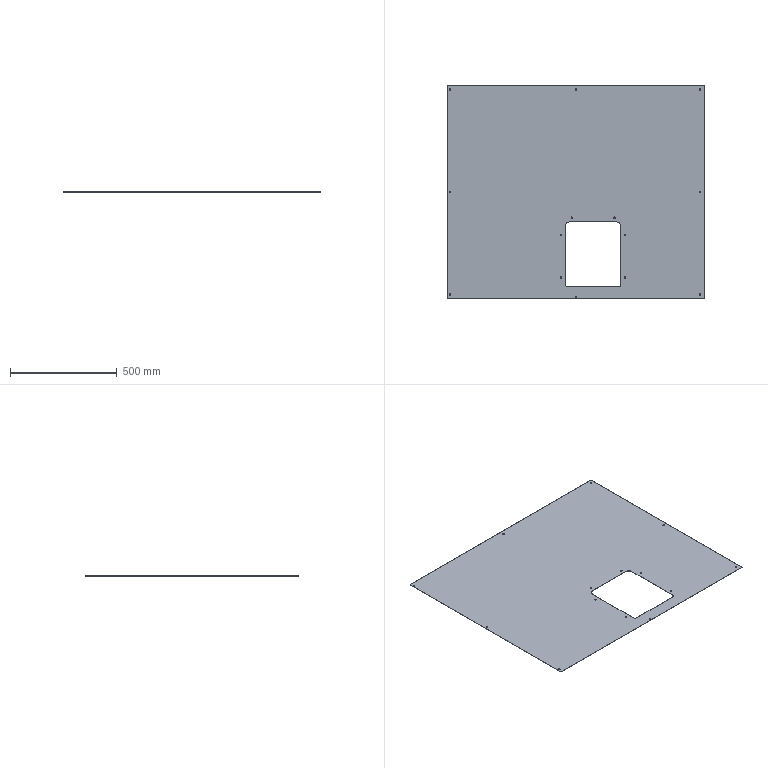Part | SolidWorks | features Fillet 3, HoleWzd 2, FlatPattern 1, ICE 1, SMBaseFlange 1, SheetMetal 1 | 1 solid | 46 faces | box 1200 x 1000 x 1.2 mm | volume 1346035 mm3 | cylinder 36 | plane 10 | commonest cylinder face diameters 6.6 x28 6 x4 10 x2 40 x2
STEP:
#1=CARTESIAN_POINT('',(-3.3,-490.,-1.2));
#2=VERTEX_POINT('',#1);
#3=CARTESIAN_POINT('',(3.3,-490.,-1.2));
#4=VERTEX_POINT('',#3);
#5=CARTESIAN_POINT('',(0.,-490.,-1.2));
#6=DIRECTION('',(0.,0.,1.));
#7=DIRECTION('',(1.,0.,0.));
#8=AXIS2_PLACEMENT_3D('',#5,#6,#7);
#9=CIRCLE('',#8,3.3);
#10=EDGE_CURVE('',#2,#4,#9,.T.);
#11=ORIENTED_EDGE('',*,*,#10,.F.);
#12=CARTESIAN_POINT('',(-3.3,-490.,0.));
#13=VERTEX_POINT('',#12);
#14=CARTESIAN_POINT('',(-3.3,-490.,0.));
#15=DIRECTION('',(0.,0.,1.));
#16=VECTOR('',#15,1000.);
#17=LINE('',#14,#16);
#18=EDGE_CURVE('',#2,#13,#17,.T.);
#19=ORIENTED_EDGE('',*,*,#18,.T.);
#20=CARTESIAN_POINT('',(3.3,-490.,0.));
#21=VERTEX_POINT('',#20);
#22=CARTESIAN_POINT('',(0.,-490.,0.));
#23=DIRECTION('',(0.,0.,1.));
#24=DIRECTION('',(1.,0.,0.));
#25=AXIS2_PLACEMENT_3D('',#22,#23,#24);
#26=CIRCLE('',#25,3.3);
#27=EDGE_CURVE('',#13,#21,#26,.T.);
#28=ORIENTED_EDGE('',*,*,#27,.T.);
#29=CARTESIAN_POINT('',(3.3,-490.,0.));
#30=DIRECTION('',(0.,0.,1.));
#31=VECTOR('',#30,1000.);
#32=LINE('',#29,#31);
#33=EDGE_CURVE('',#4,#21,#32,.T.);
#34=ORIENTED_EDGE('',*,*,#33,.F.);
#35=EDGE_LOOP('',(#11,#19,#28,#34));
#36=FACE_OUTER_BOUND('',#35,.T.);
#37=CARTESIAN_POINT('',(0.,-490.,0.));
#38=DIRECTION('',(0.,0.,1.));
#39=DIRECTION('',(1.,0.,0.));
#40=AXIS2_PLACEMENT_3D('',#37,#38,#39);
#41=CYLINDRICAL_SURFACE('',#40,3.3);
#42=ADVANCED_FACE('',(#36),#41,.F.);
#43=CARTESIAN_POINT('',(-73.3,-200.,-1.2));
#44=VERTEX_POINT('',#43);
#45=CARTESIAN_POINT('',(-66.7,-200.,-1.2));
#46=VERTEX_POINT('',#45);
#47=CARTESIAN_POINT('',(-70.,-200.,-1.2));
#48=DIRECTION('',(0.,0.,1.));
#49=DIRECTION('',(1.,0.,0.));
#50=AXIS2_PLACEMENT_3D('',#47,#48,#49);
#51=CIRCLE('',#50,3.3);
#52=EDGE_CURVE('',#44,#46,#51,.T.);
#53=ORIENTED_EDGE('',*,*,#52,.F.);
#54=CARTESIAN_POINT('',(-73.3,-200.,0.));
#55=VERTEX_POINT('',#54);
#56=CARTESIAN_POINT('',(-73.3,-200.,0.));
#57=DIRECTION('',(0.,0.,1.));
#58=VECTOR('',#57,1000.);
#59=LINE('',#56,#58);
#60=EDGE_CURVE('',#44,#55,#59,.T.);
#61=ORIENTED_EDGE('',*,*,#60,.T.);
#62=CARTESIAN_POINT('',(-66.7,-200.,0.));
#63=VERTEX_POINT('',#62);
#64=CARTESIAN_POINT('',(-70.,-200.,0.));
#65=DIRECTION('',(0.,0.,1.));
#66=DIRECTION('',(1.,0.,0.));
#67=AXIS2_PLACEMENT_3D('',#64,#65,#66);
#68=CIRCLE('',#67,3.3);
#69=EDGE_CURVE('',#55,#63,#68,.T.);
#70=ORIENTED_EDGE('',*,*,#69,.T.);
#71=CARTESIAN_POINT('',(-66.7,-200.,0.));
#72=DIRECTION('',(0.,0.,1.));
#73=VECTOR('',#72,1000.);
#74=LINE('',#71,#73);
#75=EDGE_CURVE('',#46,#63,#74,.T.);
#76=ORIENTED_EDGE('',*,*,#75,.F.);
#77=EDGE_LOOP('',(#53,#61,#70,#76));
#78=FACE_OUTER_BOUND('',#77,.T.);
#79=CARTESIAN_POINT('',(-70.,-200.,0.));
#80=DIRECTION('',(0.,0.,1.));
#81=DIRECTION('',(1.,0.,0.));
#82=AXIS2_PLACEMENT_3D('',#79,#80,#81);
#83=CYLINDRICAL_SURFACE('',#82,3.3);
#84=ADVANCED_FACE('',(#78),#83,.F.);
#85=CARTESIAN_POINT('',(-73.3,-400.,-1.2));
#86=VERTEX_POINT('',#85);
#87=CARTESIAN_POINT('',(-66.7,-400.,-1.2));
#88=VERTEX_POINT('',#87);
#89=CARTESIAN_POINT('',(-70.,-400.,-1.2));
#90=DIRECTION('',(0.,0.,1.));
#91=DIRECTION('',(1.,0.,0.));
#92=AXIS2_PLACEMENT_3D('',#89,#90,#91);
#93=CIRCLE('',#92,3.3);
#94=EDGE_CURVE('',#86,#88,#93,.T.);
#95=ORIENTED_EDGE('',*,*,#94,.F.);
#96=CARTESIAN_POINT('',(-73.3,-400.,0.));
#97=VERTEX_POINT('',#96);
#98=CARTESIAN_POINT('',(-73.3,-400.,0.));
#99=DIRECTION('',(0.,0.,1.));
#100=VECTOR('',#99,1000.);
#101=LINE('',#98,#100);
#102=EDGE_CURVE('',#86,#97,#101,.T.);
#103=ORIENTED_EDGE('',*,*,#102,.T.);
#104=CARTESIAN_POINT('',(-66.7,-400.,0.));
#105=VERTEX_POINT('',#104);
#106=CARTESIAN_POINT('',(-70.,-400.,0.));
#107=DIRECTION('',(0.,0.,1.));
#108=DIRECTION('',(1.,0.,0.));
#109=AXIS2_PLACEMENT_3D('',#106,#107,#108);
#110=CIRCLE('',#109,3.3);
#111=EDGE_CURVE('',#97,#105,#110,.T.);
#112=ORIENTED_EDGE('',*,*,#111,.T.);
#113=CARTESIAN_POINT('',(-66.7,-400.,0.));
#114=DIRECTION('',(0.,0.,1.));
#115=VECTOR('',#114,1000.);
#116=LINE('',#113,#115);
#117=EDGE_CURVE('',#88,#105,#116,.T.);
#118=ORIENTED_EDGE('',*,*,#117,.F.);
#119=EDGE_LOOP('',(#95,#103,#112,#118));
#120=FACE_OUTER_BOUND('',#119,.T.);
#121=CARTESIAN_POINT('',(-70.,-400.,0.));
#122=DIRECTION('',(0.,0.,1.));
#123=DIRECTION('',(1.,0.,0.));
#124=AXIS2_PLACEMENT_3D('',#121,#122,#123);
#125=CYLINDRICAL_SURFACE('',#124,3.3);
#126=ADVANCED_FACE('',(#120),#125,.F.);
#127=CARTESIAN_POINT('',(226.7,-200.,-1.2));
#128=VERTEX_POINT('',#127);
#129=CARTESIAN_POINT('',(233.3,-200.,-1.2));
#130=VERTEX_POINT('',#129);
#131=CARTESIAN_POINT('',(230.,-200.,-1.2));
#132=DIRECTION('',(0.,0.,1.));
#133=DIRECTION('',(1.,0.,0.));
#134=AXIS2_PLACEMENT_3D('',#131,#132,#133);
#135=CIRCLE('',#134,3.3);
#136=EDGE_CURVE('',#128,#130,#135,.T.);
#137=ORIENTED_EDGE('',*,*,#136,.F.);
#138=CARTESIAN_POINT('',(226.7,-200.,0.));
#139=VERTEX_POINT('',#138);
#140=CARTESIAN_POINT('',(226.7,-200.,0.));
#141=DIRECTION('',(0.,0.,1.));
#142=VECTOR('',#141,1000.);
#143=LINE('',#140,#142);
#144=EDGE_CURVE('',#128,#139,#143,.T.);
#145=ORIENTED_EDGE('',*,*,#144,.T.);
#146=CARTESIAN_POINT('',(233.3,-200.,0.));
#147=VERTEX_POINT('',#146);
#148=CARTESIAN_POINT('',(230.,-200.,0.));
#149=DIRECTION('',(0.,0.,1.));
#150=DIRECTION('',(1.,0.,0.));
#151=AXIS2_PLACEMENT_3D('',#148,#149,#150);
#152=CIRCLE('',#151,3.3);
#153=EDGE_CURVE('',#139,#147,#152,.T.);
#154=ORIENTED_EDGE('',*,*,#153,.T.);
#155=CARTESIAN_POINT('',(233.3,-200.,0.));
#156=DIRECTION('',(0.,0.,1.));
#157=VECTOR('',#156,1000.);
#158=LINE('',#155,#157);
#159=EDGE_CURVE('',#130,#147,#158,.T.);
#160=ORIENTED_EDGE('',*,*,#159,.F.);
#161=EDGE_LOOP('',(#137,#145,#154,#160));
#162=FACE_OUTER_BOUND('',#161,.T.);
#163=CARTESIAN_POINT('',(230.,-200.,0.));
#164=DIRECTION('',(0.,0.,1.));
#165=DIRECTION('',(1.,0.,0.));
#166=AXIS2_PLACEMENT_3D('',#163,#164,#165);
#167=CYLINDRICAL_SURFACE('',#166,3.3);
#168=ADVANCED_FACE('',(#162),#167,.F.);
#169=CARTESIAN_POINT('',(226.7,-400.,-1.2));
#170=VERTEX_POINT('',#169);
#171=CARTESIAN_POINT('',(233.3,-400.,-1.2));
#172=VERTEX_POINT('',#171);
#173=CARTESIAN_POINT('',(230.,-400.,-1.2));
#174=DIRECTION('',(0.,0.,1.));
#175=DIRECTION('',(1.,0.,0.));
#176=AXIS2_PLACEMENT_3D('',#173,#174,#175);
#177=CIRCLE('',#176,3.3);
#178=EDGE_CURVE('',#170,#172,#177,.T.);
#179=ORIENTED_EDGE('',*,*,#178,.F.);
#180=CARTESIAN_POINT('',(226.7,-400.,0.));
#181=VERTEX_POINT('',#180);
#182=CARTESIAN_POINT('',(226.7,-400.,0.));
#183=DIRECTION('',(0.,0.,1.));
#184=VECTOR('',#183,1000.);
#185=LINE('',#182,#184);
#186=EDGE_CURVE('',#170,#181,#185,.T.);
#187=ORIENTED_EDGE('',*,*,#186,.T.);
#188=CARTESIAN_POINT('',(233.3,-400.,0.));
#189=VERTEX_POINT('',#188);
#190=CARTESIAN_POINT('',(230.,-400.,0.));
#191=DIRECTION('',(0.,0.,1.));
#192=DIRECTION('',(1.,0.,0.));
#193=AXIS2_PLACEMENT_3D('',#190,#191,#192);
#194=CIRCLE('',#193,3.3);
#195=EDGE_CURVE('',#181,#189,#194,.T.);
#196=ORIENTED_EDGE('',*,*,#195,.T.);
#197=CARTESIAN_POINT('',(233.3,-400.,0.));
#198=DIRECTION('',(0.,0.,1.));
#199=VECTOR('',#198,1000.);
#200=LINE('',#197,#199);
#201=EDGE_CURVE('',#172,#189,#200,.T.);
#202=ORIENTED_EDGE('',*,*,#201,.F.);
#203=EDGE_LOOP('',(#179,#187,#196,#202));
#204=FACE_OUTER_BOUND('',#203,.T.);
#205=CARTESIAN_POINT('',(230.,-400.,0.));
#206=DIRECTION('',(0.,0.,1.));
#207=DIRECTION('',(1.,0.,0.));
#208=AXIS2_PLACEMENT_3D('',#205,#206,#207);
#209=CYLINDRICAL_SURFACE('',#208,3.3);
#210=ADVANCED_FACE('',(#204),#209,.F.);
#211=CARTESIAN_POINT('',(-23.3,-120.,-1.2));
#212=VERTEX_POINT('',#211);
#213=CARTESIAN_POINT('',(-16.7,-120.,-1.2));
#214=VERTEX_POINT('',#213);
#215=CARTESIAN_POINT('',(-20.,-120.,-1.2));
#216=DIRECTION('',(0.,0.,1.));
#217=DIRECTION('',(1.,0.,0.));
#218=AXIS2_PLACEMENT_3D('',#215,#216,#217);
#219=CIRCLE('',#218,3.3);
#220=EDGE_CURVE('',#212,#214,#219,.T.);
#221=ORIENTED_EDGE('',*,*,#220,.F.);
#222=CARTESIAN_POINT('',(-23.3,-120.,0.));
#223=VERTEX_POINT('',#222);
#224=CARTESIAN_POINT('',(-23.3,-120.,0.));
#225=DIRECTION('',(0.,0.,1.));
#226=VECTOR('',#225,1000.);
#227=LINE('',#224,#226);
#228=EDGE_CURVE('',#212,#223,#227,.T.);
#229=ORIENTED_EDGE('',*,*,#228,.T.);
#230=CARTESIAN_POINT('',(-16.7,-120.,0.));
#231=VERTEX_POINT('',#230);
#232=CARTESIAN_POINT('',(-20.,-120.,0.));
#233=DIRECTION('',(0.,0.,1.));
#234=DIRECTION('',(1.,0.,0.));
#235=AXIS2_PLACEMENT_3D('',#232,#233,#234);
#236=CIRCLE('',#235,3.3);
#237=EDGE_CURVE('',#223,#231,#236,.T.);
#238=ORIENTED_EDGE('',*,*,#237,.T.);
#239=CARTESIAN_POINT('',(-16.7,-120.,0.));
#240=DIRECTION('',(0.,0.,1.));
#241=VECTOR('',#240,1000.);
#242=LINE('',#239,#241);
#243=EDGE_CURVE('',#214,#231,#242,.T.);
#244=ORIENTED_EDGE('',*,*,#243,.F.);
#245=EDGE_LOOP('',(#221,#229,#238,#244));
#246=FACE_OUTER_BOUND('',#245,.T.);
#247=CARTESIAN_POINT('',(-20.,-120.,0.));
#248=DIRECTION('',(0.,0.,1.));
#249=DIRECTION('',(1.,0.,0.));
#250=AXIS2_PLACEMENT_3D('',#247,#248,#249);
#251=CYLINDRICAL_SURFACE('',#250,3.3);
#252=ADVANCED_FACE('',(#246),#251,.F.);
#253=CARTESIAN_POINT('',(176.7,-120.,-1.2));
#254=VERTEX_POINT('',#253);
#255=CARTESIAN_POINT('',(183.3,-120.,-1.2));
#256=VERTEX_POINT('',#255);
#257=CARTESIAN_POINT('',(180.,-120.,-1.2));
#258=DIRECTION('',(0.,0.,1.));
#259=DIRECTION('',(1.,0.,0.));
#260=AXIS2_PLACEMENT_3D('',#257,#258,#259);
#261=CIRCLE('',#260,3.3);
#262=EDGE_CURVE('',#254,#256,#261,.T.);
#263=ORIENTED_EDGE('',*,*,#262,.F.);
#264=CARTESIAN_POINT('',(176.7,-120.,0.));
#265=VERTEX_POINT('',#264);
#266=CARTESIAN_POINT('',(176.7,-120.,0.));
#267=DIRECTION('',(0.,0.,1.));
#268=VECTOR('',#267,1000.);
#269=LINE('',#266,#268);
#270=EDGE_CURVE('',#254,#265,#269,.T.);
#271=ORIENTED_EDGE('',*,*,#270,.T.);
#272=CARTESIAN_POINT('',(183.3,-120.,0.));
#273=VERTEX_POINT('',#272);
#274=CARTESIAN_POINT('',(180.,-120.,0.));
#275=DIRECTION('',(0.,0.,1.));
#276=DIRECTION('',(1.,0.,0.));
#277=AXIS2_PLACEMENT_3D('',#274,#275,#276);
#278=CIRCLE('',#277,3.3);
#279=EDGE_CURVE('',#265,#273,#278,.T.);
#280=ORIENTED_EDGE('',*,*,#279,.T.);
#281=CARTESIAN_POINT('',(183.3,-120.,0.));
#282=DIRECTION('',(0.,0.,1.));
#283=VECTOR('',#282,1000.);
#284=LINE('',#281,#283);
#285=EDGE_CURVE('',#256,#273,#284,.T.);
#286=ORIENTED_EDGE('',*,*,#285,.F.);
#287=EDGE_LOOP('',(#263,#271,#280,#286));
#288=FACE_OUTER_BOUND('',#287,.T.);
#289=CARTESIAN_POINT('',(180.,-120.,0.));
#290=DIRECTION('',(0.,0.,1.));
#291=DIRECTION('',(1.,0.,0.));
#292=AXIS2_PLACEMENT_3D('',#289,#290,#291);
#293=CYLINDRICAL_SURFACE('',#292,3.3);
#294=ADVANCED_FACE('',(#288),#293,.F.);
#295=CARTESIAN_POINT('',(-593.3,480.,-1.2));
#296=VERTEX_POINT('',#295);
#297=CARTESIAN_POINT('',(-586.7,480.,-1.2));
#298=VERTEX_POINT('',#297);
#299=CARTESIAN_POINT('',(-590.,480.,-1.2));
#300=DIRECTION('',(0.,0.,1.));
#301=DIRECTION('',(1.,0.,0.));
#302=AXIS2_PLACEMENT_3D('',#299,#300,#301);
#303=CIRCLE('',#302,3.3);
#304=EDGE_CURVE('',#296,#298,#303,.T.);
#305=ORIENTED_EDGE('',*,*,#304,.F.);
#306=CARTESIAN_POINT('',(-593.3,480.,0.));
#307=VERTEX_POINT('',#306);
#308=CARTESIAN_POINT('',(-593.3,480.,0.));
#309=DIRECTION('',(0.,0.,1.));
#310=VECTOR('',#309,1000.);
#311=LINE('',#308,#310);
#312=EDGE_CURVE('',#296,#307,#311,.T.);
#313=ORIENTED_EDGE('',*,*,#312,.T.);
#314=CARTESIAN_POINT('',(-586.7,480.,0.));
#315=VERTEX_POINT('',#314);
#316=CARTESIAN_POINT('',(-590.,480.,0.));
#317=DIRECTION('',(0.,0.,1.));
#318=DIRECTION('',(1.,0.,0.));
#319=AXIS2_PLACEMENT_3D('',#316,#317,#318);
#320=CIRCLE('',#319,3.3);
#321=EDGE_CURVE('',#307,#315,#320,.T.);
#322=ORIENTED_EDGE('',*,*,#321,.T.);
#323=CARTESIAN_POINT('',(-586.7,480.,0.));
#324=DIRECTION('',(0.,0.,1.));
#325=VECTOR('',#324,1000.);
#326=LINE('',#323,#325);
#327=EDGE_CURVE('',#298,#315,#326,.T.);
#328=ORIENTED_EDGE('',*,*,#327,.F.);
#329=EDGE_LOOP('',(#305,#313,#322,#328));
#330=FACE_OUTER_BOUND('',#329,.T.);
#331=CARTESIAN_POINT('',(-590.,480.,0.));
#332=DIRECTION('',(0.,0.,1.));
#333=DIRECTION('',(1.,0.,0.));
#334=AXIS2_PLACEMENT_3D('',#331,#332,#333);
#335=CYLINDRICAL_SURFACE('',#334,3.3);
#336=ADVANCED_FACE('',(#330),#335,.F.);
#337=CARTESIAN_POINT('',(-593.3,0.,-1.2));
#338=VERTEX_POINT('',#337);
#339=CARTESIAN_POINT('',(-586.7,0.,-1.2));
#340=VERTEX_POINT('',#339);
#341=CARTESIAN_POINT('',(-590.,0.,-1.2));
#342=DIRECTION('',(0.,0.,1.));
#343=DIRECTION('',(1.,0.,0.));
#344=AXIS2_PLACEMENT_3D('',#341,#342,#343);
#345=CIRCLE('',#344,3.3);
#346=EDGE_CURVE('',#338,#340,#345,.T.);
#347=ORIENTED_EDGE('',*,*,#346,.F.);
#348=CARTESIAN_POINT('',(-593.3,0.,0.));
#349=VERTEX_POINT('',#348);
#350=CARTESIAN_POINT('',(-593.3,0.,0.));
#351=DIRECTION('',(0.,0.,1.));
#352=VECTOR('',#351,1000.);
#353=LINE('',#350,#352);
#354=EDGE_CURVE('',#338,#349,#353,.T.);
#355=ORIENTED_EDGE('',*,*,#354,.T.);
#356=CARTESIAN_POINT('',(-586.7,0.,0.));
#357=VERTEX_POINT('',#356);
#358=CARTESIAN_POINT('',(-590.,0.,0.));
#359=DIRECTION('',(0.,0.,1.));
#360=DIRECTION('',(1.,0.,0.));
#361=AXIS2_PLACEMENT_3D('',#358,#359,#360);
#362=CIRCLE('',#361,3.3);
#363=EDGE_CURVE('',#349,#357,#362,.T.);
#364=ORIENTED_EDGE('',*,*,#363,.T.);
#365=CARTESIAN_POINT('',(-586.7,0.,0.));
#366=DIRECTION('',(0.,0.,1.));
#367=VECTOR('',#366,1000.);
#368=LINE('',#365,#367);
#369=EDGE_CURVE('',#340,#357,#368,.T.);
#370=ORIENTED_EDGE('',*,*,#369,.F.);
#371=EDGE_LOOP('',(#347,#355,#364,#370));
#372=FACE_OUTER_BOUND('',#371,.T.);
#373=CARTESIAN_POINT('',(-590.,0.,0.));
#374=DIRECTION('',(0.,0.,1.));
#375=DIRECTION('',(1.,0.,0.));
#376=AXIS2_PLACEMENT_3D('',#373,#374,#375);
#377=CYLINDRICAL_SURFACE('',#376,3.3);
#378=ADVANCED_FACE('',(#372),#377,.F.);
#379=CARTESIAN_POINT('',(-593.3,-480.,-1.2));
#380=VERTEX_POINT('',#379);
#381=CARTESIAN_POINT('',(-586.7,-480.,-1.2));
#382=VERTEX_POINT('',#381);
#383=CARTESIAN_POINT('',(-590.,-480.,-1.2));
#384=DIRECTION('',(0.,0.,1.));
#385=DIRECTION('',(1.,0.,0.));
#386=AXIS2_PLACEMENT_3D('',#383,#384,#385);
#387=CIRCLE('',#386,3.3);
#388=EDGE_CURVE('',#380,#382,#387,.T.);
#389=ORIENTED_EDGE('',*,*,#388,.F.);
#390=CARTESIAN_POINT('',(-593.3,-480.,0.));
#391=VERTEX_POINT('',#390);
#392=CARTESIAN_POINT('',(-593.3,-480.,0.));
#393=DIRECTION('',(0.,0.,1.));
#394=VECTOR('',#393,1000.);
#395=LINE('',#392,#394);
#396=EDGE_CURVE('',#380,#391,#395,.T.);
#397=ORIENTED_EDGE('',*,*,#396,.T.);
#398=CARTESIAN_POINT('',(-586.7,-480.,0.));
#399=VERTEX_POINT('',#398);
#400=CARTESIAN_POINT('',(-590.,-480.,0.));
#401=DIRECTION('',(0.,0.,1.));
#402=DIRECTION('',(1.,0.,0.));
#403=AXIS2_PLACEMENT_3D('',#400,#401,#402);
#404=CIRCLE('',#403,3.3);
#405=EDGE_CURVE('',#391,#399,#404,.T.);
#406=ORIENTED_EDGE('',*,*,#405,.T.);
#407=CARTESIAN_POINT('',(-586.7,-480.,0.));
#408=DIRECTION('',(0.,0.,1.));
#409=VECTOR('',#408,1000.);
#410=LINE('',#407,#409);
#411=EDGE_CURVE('',#382,#399,#410,.T.);
#412=ORIENTED_EDGE('',*,*,#411,.F.);
#413=EDGE_LOOP('',(#389,#397,#406,#412));
#414=FACE_OUTER_BOUND('',#413,.T.);
#415=CARTESIAN_POINT('',(-590.,-480.,0.));
#416=DIRECTION('',(0.,0.,1.));
#417=DIRECTION('',(1.,0.,0.));
#418=AXIS2_PLACEMENT_3D('',#415,#416,#417);
#419=CYLINDRICAL_SURFACE('',#418,3.3);
#420=ADVANCED_FACE('',(#414),#419,.F.);
#421=CARTESIAN_POINT('',(-3.3,480.,-1.2));
#422=VERTEX_POINT('',#421);
#423=CARTESIAN_POINT('',(3.3,480.,-1.2));
#424=VERTEX_POINT('',#423);
#425=CARTESIAN_POINT('',(0.,480.,-1.2));
#426=DIRECTION('',(0.,0.,1.));
#427=DIRECTION('',(1.,0.,0.));
#428=AXIS2_PLACEMENT_3D('',#425,#426,#427);
#429=CIRCLE('',#428,3.3);
#430=EDGE_CURVE('',#422,#424,#429,.T.);
#431=ORIENTED_EDGE('',*,*,#430,.F.);
#432=CARTESIAN_POINT('',(-3.3,480.,0.));
#433=VERTEX_POINT('',#432);
#434=CARTESIAN_POINT('',(-3.3,480.,0.));
#435=DIRECTION('',(0.,0.,1.));
#436=VECTOR('',#435,1000.);
#437=LINE('',#434,#436);
#438=EDGE_CURVE('',#422,#433,#437,.T.);
#439=ORIENTED_EDGE('',*,*,#438,.T.);
#440=CARTESIAN_POINT('',(3.3,480.,0.));
#441=VERTEX_POINT('',#440);
#442=CARTESIAN_POINT('',(0.,480.,0.));
#443=DIRECTION('',(0.,0.,1.));
#444=DIRECTION('',(1.,0.,0.));
#445=AXIS2_PLACEMENT_3D('',#442,#443,#444);
#446=CIRCLE('',#445,3.3);
#447=EDGE_CURVE('',#433,#441,#446,.T.);
#448=ORIENTED_EDGE('',*,*,#447,.T.);
#449=CARTESIAN_POINT('',(3.3,480.,0.));
#450=DIRECTION('',(0.,0.,1.));
#451=VECTOR('',#450,1000.);
#452=LINE('',#449,#451);
#453=EDGE_CURVE('',#424,#441,#452,.T.);
#454=ORIENTED_EDGE('',*,*,#453,.F.);
#455=EDGE_LOOP('',(#431,#439,#448,#454));
#456=FACE_OUTER_BOUND('',#455,.T.);
#457=CARTESIAN_POINT('',(0.,480.,0.));
#458=DIRECTION('',(0.,0.,1.));
#459=DIRECTION('',(1.,0.,0.));
#460=AXIS2_PLACEMENT_3D('',#457,#458,#459);
#461=CYLINDRICAL_SURFACE('',#460,3.3);
#462=ADVANCED_FACE('',(#456),#461,.F.);
#463=CARTESIAN_POINT('',(576.7,480.,-1.2));
#464=VERTEX_POINT('',#463);
#465=CARTESIAN_POINT('',(583.3,480.,-1.2));
#466=VERTEX_POINT('',#465);
#467=CARTESIAN_POINT('',(580.,480.,-1.2));
#468=DIRECTION('',(0.,0.,1.));
#469=DIRECTION('',(1.,0.,0.));
#470=AXIS2_PLACEMENT_3D('',#467,#468,#469);
#471=CIRCLE('',#470,3.3);
#472=EDGE_CURVE('',#464,#466,#471,.T.);
#473=ORIENTED_EDGE('',*,*,#472,.F.);
#474=CARTESIAN_POINT('',(576.7,480.,0.));
#475=VERTEX_POINT('',#474);
#476=CARTESIAN_POINT('',(576.7,480.,0.));
#477=DIRECTION('',(0.,0.,1.));
#478=VECTOR('',#477,1000.);
#479=LINE('',#476,#478);
#480=EDGE_CURVE('',#464,#475,#479,.T.);
#481=ORIENTED_EDGE('',*,*,#480,.T.);
#482=CARTESIAN_POINT('',(583.3,480.,0.));
#483=VERTEX_POINT('',#482);
#484=CARTESIAN_POINT('',(580.,480.,0.));
#485=DIRECTION('',(0.,0.,1.));
#486=DIRECTION('',(1.,0.,0.));
#487=AXIS2_PLACEMENT_3D('',#484,#485,#486);
#488=CIRCLE('',#487,3.3);
#489=EDGE_CURVE('',#475,#483,#488,.T.);
#490=ORIENTED_EDGE('',*,*,#489,.T.);
#491=CARTESIAN_POINT('',(583.3,480.,0.));
#492=DIRECTION('',(0.,0.,1.));
#493=VECTOR('',#492,1000.);
#494=LINE('',#491,#493);
#495=EDGE_CURVE('',#466,#483,#494,.T.);
#496=ORIENTED_EDGE('',*,*,#495,.F.);
#497=EDGE_LOOP('',(#473,#481,#490,#496));
#498=FACE_OUTER_BOUND('',#497,.T.);
#499=CARTESIAN_POINT('',(580.,480.,0.));
#500=DIRECTION('',(0.,0.,1.));
#501=DIRECTION('',(1.,0.,0.));
#502=AXIS2_PLACEMENT_3D('',#499,#500,#501);
#503=CYLINDRICAL_SURFACE('',#502,3.3);
#504=ADVANCED_FACE('',(#498),#503,.F.);
#505=CARTESIAN_POINT('',(576.7,-480.,-1.2));
#506=VERTEX_POINT('',#505);
#507=CARTESIAN_POINT('',(583.3,-480.,-1.2));
#508=VERTEX_POINT('',#507);
#509=CARTESIAN_POINT('',(580.,-480.,-1.2));
#510=DIRECTION('',(0.,0.,1.));
#511=DIRECTION('',(1.,0.,0.));
#512=AXIS2_PLACEMENT_3D('',#509,#510,#511);
#513=CIRCLE('',#512,3.3);
#514=EDGE_CURVE('',#506,#508,#513,.T.);
#515=ORIENTED_EDGE('',*,*,#514,.F.);
#516=CARTESIAN_POINT('',(576.7,-480.,0.));
#517=VERTEX_POINT('',#516);
#518=CARTESIAN_POINT('',(576.7,-480.,0.));
#519=DIRECTION('',(0.,0.,1.));
#520=VECTOR('',#519,1000.);
#521=LINE('',#518,#520);
#522=EDGE_CURVE('',#506,#517,#521,.T.);
#523=ORIENTED_EDGE('',*,*,#522,.T.);
#524=CARTESIAN_POINT('',(583.3,-480.,0.));
#525=VERTEX_POINT('',#524);
#526=CARTESIAN_POINT('',(580.,-480.,0.));
#527=DIRECTION('',(0.,0.,1.));
#528=DIRECTION('',(1.,0.,0.));
#529=AXIS2_PLACEMENT_3D('',#526,#527,#528);
#530=CIRCLE('',#529,3.3);
#531=EDGE_CURVE('',#517,#525,#530,.T.);
#532=ORIENTED_EDGE('',*,*,#531,.T.);
#533=CARTESIAN_POINT('',(583.3,-480.,0.));
#534=DIRECTION('',(0.,0.,1.));
#535=VECTOR('',#534,1000.);
#536=LINE('',#533,#535);
#537=EDGE_CURVE('',#508,#525,#536,.T.);
#538=ORIENTED_EDGE('',*,*,#537,.F.);
#539=EDGE_LOOP('',(#515,#523,#532,#538));
#540=FACE_OUTER_BOUND('',#539,.T.);
#541=CARTESIAN_POINT('',(580.,-480.,0.));
#542=DIRECTION('',(0.,0.,1.));
#543=DIRECTION('',(1.,0.,0.));
#544=AXIS2_PLACEMENT_3D('',#541,#542,#543);
#545=CYLINDRICAL_SURFACE('',#544,3.3);
#546=ADVANCED_FACE('',(#540),#545,.F.);
#547=CARTESIAN_POINT('',(576.7,0.,-1.2));
#548=VERTEX_POINT('',#547);
#549=CARTESIAN_POINT('',(583.3,0.,-1.2));
#550=VERTEX_POINT('',#549);
#551=CARTESIAN_POINT('',(580.,0.,-1.2));
#552=DIRECTION('',(0.,0.,1.));
#553=DIRECTION('',(1.,0.,0.));
#554=AXIS2_PLACEMENT_3D('',#551,#552,#553);
#555=CIRCLE('',#554,3.3);
#556=EDGE_CURVE('',#548,#550,#555,.T.);
#557=ORIENTED_EDGE('',*,*,#556,.F.);
#558=CARTESIAN_POINT('',(576.7,0.,0.));
#559=VERTEX_POINT('',#558);
#560=CARTESIAN_POINT('',(576.7,0.,0.));
#561=DIRECTION('',(0.,0.,1.));
#562=VECTOR('',#561,1000.);
#563=LINE('',#560,#562);
#564=EDGE_CURVE('',#548,#559,#563,.T.);
#565=ORIENTED_EDGE('',*,*,#564,.T.);
#566=CARTESIAN_POINT('',(583.3,0.,0.));
#567=VERTEX_POINT('',#566);
#568=CARTESIAN_POINT('',(580.,0.,0.));
#569=DIRECTION('',(0.,0.,1.));
#570=DIRECTION('',(1.,0.,0.));
#571=AXIS2_PLACEMENT_3D('',#568,#569,#570);
#572=CIRCLE('',#571,3.3);
#573=EDGE_CURVE('',#559,#567,#572,.T.);
#574=ORIENTED_EDGE('',*,*,#573,.T.);
#575=CARTESIAN_POINT('',(583.3,0.,0.));
#576=DIRECTION('',(0.,0.,1.));
#577=VECTOR('',#576,1000.);
#578=LINE('',#575,#577);
#579=EDGE_CURVE('',#550,#567,#578,.T.);
#580=ORIENTED_EDGE('',*,*,#579,.F.);
#581=EDGE_LOOP('',(#557,#565,#574,#580));
#582=FACE_OUTER_BOUND('',#581,.T.);
#583=CARTESIAN_POINT('',(580.,0.,0.));
#584=DIRECTION('',(0.,0.,1.));
#585=DIRECTION('',(1.,0.,0.));
#586=AXIS2_PLACEMENT_3D('',#583,#584,#585);
#587=CYLINDRICAL_SURFACE('',#586,3.3);
#588=ADVANCED_FACE('',(#582),#587,.F.);
#589=CARTESIAN_POINT('',(600.,-497.,0.));
#590=VERTEX_POINT('',#589);
#591=CARTESIAN_POINT('',(600.,497.,0.));
#592=VERTEX_POINT('',#591);
#593=CARTESIAN_POINT('',(600.,500.,0.));
#594=DIRECTION('',(0.,1.,0.));
#595=VECTOR('',#594,1000.);
#596=LINE('',#593,#595);
#597=EDGE_CURVE('',#590,#592,#596,.T.);
#598=ORIENTED_EDGE('',*,*,#597,.F.);
#599=CARTESIAN_POINT('',(600.,-497.,-1.2));
#600=VERTEX_POINT('',#599);
#601=CARTESIAN_POINT('',(600.,-497.,-1.2));
#602=DIRECTION('',(0.,0.,-1.));
#603=VECTOR('',#602,1000.);
#604=LINE('',#601,#603);
#605=EDGE_CURVE('',#590,#600,#604,.T.);
#606=ORIENTED_EDGE('',*,*,#605,.T.);
#607=CARTESIAN_POINT('',(600.,497.,-1.2));
#608=VERTEX_POINT('',#607);
#609=CARTESIAN_POINT('',(600.,500.,-1.2));
#610=DIRECTION('',(0.,1.,0.));
#611=VECTOR('',#610,1000.);
#612=LINE('',#609,#611);
#613=EDGE_CURVE('',#600,#608,#612,.T.);
#614=ORIENTED_EDGE('',*,*,#613,.T.);
#615=CARTESIAN_POINT('',(600.,497.,-1.2));
#616=DIRECTION('',(0.,0.,1.));
#617=VECTOR('',#616,1000.);
#618=LINE('',#615,#617);
#619=EDGE_CURVE('',#608,#592,#618,.T.);
#620=ORIENTED_EDGE('',*,*,#619,.T.);
#621=EDGE_LOOP('',(#598,#606,#614,#620));
#622=FACE_OUTER_BOUND('',#621,.T.);
#623=CARTESIAN_POINT('',(600.,500.,-1.2));
#624=DIRECTION('',(1.,0.,0.));
#625=DIRECTION('',(0.,1.,0.));
#626=AXIS2_PLACEMENT_3D('',#623,#624,#625);
#627=PLANE('',#626);
#628=ADVANCED_FACE('',(#622),#627,.T.);
#629=CARTESIAN_POINT('',(-597.,-500.,-1.2));
#630=VERTEX_POINT('',#629);
#631=CARTESIAN_POINT('',(597.,-500.,-1.2));
#632=VERTEX_POINT('',#631);
#633=CARTESIAN_POINT('',(-600.,-500.,-1.2));
#634=DIRECTION('',(1.,0.,0.));
#635=VECTOR('',#634,1000.);
#636=LINE('',#633,#635);
#637=EDGE_CURVE('',#630,#632,#636,.T.);
#638=ORIENTED_EDGE('',*,*,#637,.T.);
#639=CARTESIAN_POINT('',(597.,-500.,0.));
#640=VERTEX_POINT('',#639);
#641=CARTESIAN_POINT('',(597.,-500.,-1.2));
#642=DIRECTION('',(0.,0.,1.));
#643=VECTOR('',#642,1000.);
#644=LINE('',#641,#643);
#645=EDGE_CURVE('',#632,#640,#644,.T.);
#646=ORIENTED_EDGE('',*,*,#645,.T.);
#647=CARTESIAN_POINT('',(-597.,-500.,0.));
#648=VERTEX_POINT('',#647);
#649=CARTESIAN_POINT('',(-600.,-500.,0.));
#650=DIRECTION('',(1.,0.,0.));
#651=VECTOR('',#650,1000.);
#652=LINE('',#649,#651);
#653=EDGE_CURVE('',#648,#640,#652,.T.);
#654=ORIENTED_EDGE('',*,*,#653,.F.);
#655=CARTESIAN_POINT('',(-597.,-500.,-1.2));
#656=DIRECTION('',(0.,0.,-1.));
#657=VECTOR('',#656,1000.);
#658=LINE('',#655,#657);
#659=EDGE_CURVE('',#648,#630,#658,.T.);
#660=ORIENTED_EDGE('',*,*,#659,.T.);
#661=EDGE_LOOP('',(#638,#646,#654,#660));
#662=FACE_OUTER_BOUND('',#661,.T.);
#663=CARTESIAN_POINT('',(-600.,-500.,-1.2));
#664=DIRECTION('',(0.,-1.,0.));
#665=DIRECTION('',(0.,0.,-1.));
#666=AXIS2_PLACEMENT_3D('',#663,#664,#665);
#667=PLANE('',#666);
#668=ADVANCED_FACE('',(#662),#667,.T.);
#669=CARTESIAN_POINT('',(-600.,497.,-1.2));
#670=VERTEX_POINT('',#669);
#671=CARTESIAN_POINT('',(-600.,-497.,-1.2));
#672=VERTEX_POINT('',#671);
#673=CARTESIAN_POINT('',(-600.,500.,-1.2));
#674=DIRECTION('',(0.,-1.,0.));
#675=VECTOR('',#674,1000.);
#676=LINE('',#673,#675);
#677=EDGE_CURVE('',#670,#672,#676,.T.);
#678=ORIENTED_EDGE('',*,*,#677,.T.);
#679=CARTESIAN_POINT('',(-600.,-497.,0.));
#680=VERTEX_POINT('',#679);
#681=CARTESIAN_POINT('',(-600.,-497.,-1.2));
#682=DIRECTION('',(0.,0.,1.));
#683=VECTOR('',#682,1000.);
#684=LINE('',#681,#683);
#685=EDGE_CURVE('',#672,#680,#684,.T.);
#686=ORIENTED_EDGE('',*,*,#685,.T.);
#687=CARTESIAN_POINT('',(-600.,497.,0.));
#688=VERTEX_POINT('',#687);
#689=CARTESIAN_POINT('',(-600.,500.,0.));
#690=DIRECTION('',(0.,-1.,0.));
#691=VECTOR('',#690,1000.);
#692=LINE('',#689,#691);
#693=EDGE_CURVE('',#688,#680,#692,.T.);
#694=ORIENTED_EDGE('',*,*,#693,.F.);
#695=CARTESIAN_POINT('',(-600.,497.,-1.2));
#696=DIRECTION('',(0.,0.,-1.));
#697=VECTOR('',#696,1000.);
#698=LINE('',#695,#697);
#699=EDGE_CURVE('',#688,#670,#698,.T.);
#700=ORIENTED_EDGE('',*,*,#699,.T.);
#701=EDGE_LOOP('',(#678,#686,#694,#700));
#702=FACE_OUTER_BOUND('',#701,.T.);
#703=CARTESIAN_POINT('',(-600.,500.,-1.2));
#704=DIRECTION('',(-1.,0.,0.));
#705=DIRECTION('',(0.,-1.,0.));
#706=AXIS2_PLACEMENT_3D('',#703,#704,#705);
#707=PLANE('',#706);
#708=ADVANCED_FACE('',(#702),#707,.T.);
#709=CARTESIAN_POINT('',(597.,500.,0.));
#710=VERTEX_POINT('',#709);
#711=CARTESIAN_POINT('',(-597.,500.,0.));
#712=VERTEX_POINT('',#711);
#713=CARTESIAN_POINT('',(-600.,500.,0.));
#714=DIRECTION('',(-1.,0.,0.));
#715=VECTOR('',#714,1000.);
#716=LINE('',#713,#715);
#717=EDGE_CURVE('',#710,#712,#716,.T.);
#718=ORIENTED_EDGE('',*,*,#717,.F.);
#719=CARTESIAN_POINT('',(597.,500.,-1.2));
#720=VERTEX_POINT('',#719);
#721=CARTESIAN_POINT('',(597.,500.,-1.2));
#722=DIRECTION('',(0.,0.,-1.));
#723=VECTOR('',#722,1000.);
#724=LINE('',#721,#723);
#725=EDGE_CURVE('',#710,#720,#724,.T.);
#726=ORIENTED_EDGE('',*,*,#725,.T.);
#727=CARTESIAN_POINT('',(-597.,500.,-1.2));
#728=VERTEX_POINT('',#727);
#729=CARTESIAN_POINT('',(-600.,500.,-1.2));
#730=DIRECTION('',(-1.,0.,0.));
#731=VECTOR('',#730,1000.);
#732=LINE('',#729,#731);
#733=EDGE_CURVE('',#720,#728,#732,.T.);
#734=ORIENTED_EDGE('',*,*,#733,.T.);
#735=CARTESIAN_POINT('',(-597.,500.,-1.2));
#736=DIRECTION('',(0.,0.,1.));
#737=VECTOR('',#736,1000.);
#738=LINE('',#735,#737);
#739=EDGE_CURVE('',#728,#712,#738,.T.);
#740=ORIENTED_EDGE('',*,*,#739,.T.);
#741=EDGE_LOOP('',(#718,#726,#734,#740));
#742=FACE_OUTER_BOUND('',#741,.T.);
#743=CARTESIAN_POINT('',(-600.,500.,-1.2));
#744=DIRECTION('',(0.,1.,0.));
#745=DIRECTION('',(0.,0.,1.));
#746=AXIS2_PLACEMENT_3D('',#743,#744,#745);
#747=PLANE('',#746);
#748=ADVANCED_FACE('',(#742),#747,.T.);
#749=CARTESIAN_POINT('',(0.,-490.,-1.2));
#750=DIRECTION('',(0.,0.,1.));
#751=DIRECTION('',(1.,0.,0.));
#752=AXIS2_PLACEMENT_3D('',#749,#750,#751);
#753=CIRCLE('',#752,3.3);
#754=EDGE_CURVE('',#4,#2,#753,.T.);
#755=ORIENTED_EDGE('',*,*,#754,.T.);
#756=ORIENTED_EDGE('',*,*,#10,.T.);
#757=EDGE_LOOP('',(#755,#756));
#758=FACE_BOUND('',#757,.T.);
#759=CARTESIAN_POINT('',(-70.,-200.,-1.2));
#760=DIRECTION('',(0.,0.,1.));
#761=DIRECTION('',(1.,0.,0.));
#762=AXIS2_PLACEMENT_3D('',#759,#760,#761);
#763=CIRCLE('',#762,3.3);
#764=EDGE_CURVE('',#46,#44,#763,.T.);
#765=ORIENTED_EDGE('',*,*,#764,.T.);
#766=ORIENTED_EDGE('',*,*,#52,.T.);
#767=EDGE_LOOP('',(#765,#766));
#768=FACE_BOUND('',#767,.T.);
#769=CARTESIAN_POINT('',(-70.,-400.,-1.2));
#770=DIRECTION('',(0.,0.,1.));
#771=DIRECTION('',(1.,0.,0.));
#772=AXIS2_PLACEMENT_3D('',#769,#770,#771);
#773=CIRCLE('',#772,3.3);
#774=EDGE_CURVE('',#88,#86,#773,.T.);
#775=ORIENTED_EDGE('',*,*,#774,.T.);
#776=ORIENTED_EDGE('',*,*,#94,.T.);
#777=EDGE_LOOP('',(#775,#776));
#778=FACE_BOUND('',#777,.T.);
#779=CARTESIAN_POINT('',(230.,-200.,-1.2));
#780=DIRECTION('',(0.,0.,1.));
#781=DIRECTION('',(1.,0.,0.));
#782=AXIS2_PLACEMENT_3D('',#779,#780,#781);
#783=CIRCLE('',#782,3.3);
#784=EDGE_CURVE('',#130,#128,#783,.T.);
#785=ORIENTED_EDGE('',*,*,#784,.T.);
#786=ORIENTED_EDGE('',*,*,#136,.T.);
#787=EDGE_LOOP('',(#785,#786));
#788=FACE_BOUND('',#787,.T.);
#789=CARTESIAN_POINT('',(230.,-400.,-1.2));
#790=DIRECTION('',(0.,0.,1.));
#791=DIRECTION('',(1.,0.,0.));
#792=AXIS2_PLACEMENT_3D('',#789,#790,#791);
#793=CIRCLE('',#792,3.3);
#794=EDGE_CURVE('',#172,#170,#793,.T.);
#795=ORIENTED_EDGE('',*,*,#794,.T.);
#796=ORIENTED_EDGE('',*,*,#178,.T.);
#797=EDGE_LOOP('',(#795,#796));
#798=FACE_BOUND('',#797,.T.);
#799=CARTESIAN_POINT('',(-20.,-120.,-1.2));
#800=DIRECTION('',(0.,0.,1.));
#801=DIRECTION('',(1.,0.,0.));
#802=AXIS2_PLACEMENT_3D('',#799,#800,#801);
#803=CIRCLE('',#802,3.3);
#804=EDGE_CURVE('',#214,#212,#803,.T.);
#805=ORIENTED_EDGE('',*,*,#804,.T.);
#806=ORIENTED_EDGE('',*,*,#220,.T.);
#807=EDGE_LOOP('',(#805,#806));
#808=FACE_BOUND('',#807,.T.);
#809=CARTESIAN_POINT('',(180.,-120.,-1.2));
#810=DIRECTION('',(0.,0.,1.));
#811=DIRECTION('',(1.,0.,0.));
#812=AXIS2_PLACEMENT_3D('',#809,#810,#811);
#813=CIRCLE('',#812,3.3);
#814=EDGE_CURVE('',#256,#254,#813,.T.);
#815=ORIENTED_EDGE('',*,*,#814,.T.);
#816=ORIENTED_EDGE('',*,*,#262,.T.);
#817=EDGE_LOOP('',(#815,#816));
#818=FACE_BOUND('',#817,.T.);
#819=CARTESIAN_POINT('',(-590.,480.,-1.2));
#820=DIRECTION('',(0.,0.,1.));
#821=DIRECTION('',(1.,0.,0.));
#822=AXIS2_PLACEMENT_3D('',#819,#820,#821);
#823=CIRCLE('',#822,3.3);
#824=EDGE_CURVE('',#298,#296,#823,.T.);
#825=ORIENTED_EDGE('',*,*,#824,.T.);
#826=ORIENTED_EDGE('',*,*,#304,.T.);
#827=EDGE_LOOP('',(#825,#826));
#828=FACE_BOUND('',#827,.T.);
#829=CARTESIAN_POINT('',(-590.,0.,-1.2));
#830=DIRECTION('',(0.,0.,1.));
#831=DIRECTION('',(1.,0.,0.));
#832=AXIS2_PLACEMENT_3D('',#829,#830,#831);
#833=CIRCLE('',#832,3.3);
#834=EDGE_CURVE('',#340,#338,#833,.T.);
#835=ORIENTED_EDGE('',*,*,#834,.T.);
#836=ORIENTED_EDGE('',*,*,#346,.T.);
#837=EDGE_LOOP('',(#835,#836));
#838=FACE_BOUND('',#837,.T.);
#839=CARTESIAN_POINT('',(-590.,-480.,-1.2));
#840=DIRECTION('',(0.,0.,1.));
#841=DIRECTION('',(1.,0.,0.));
#842=AXIS2_PLACEMENT_3D('',#839,#840,#841);
#843=CIRCLE('',#842,3.3);
#844=EDGE_CURVE('',#382,#380,#843,.T.);
#845=ORIENTED_EDGE('',*,*,#844,.T.);
#846=ORIENTED_EDGE('',*,*,#388,.T.);
#847=EDGE_LOOP('',(#845,#846));
#848=FACE_BOUND('',#847,.T.);
#849=CARTESIAN_POINT('',(0.,480.,-1.2));
#850=DIRECTION('',(0.,0.,1.));
#851=DIRECTION('',(1.,0.,0.));
#852=AXIS2_PLACEMENT_3D('',#849,#850,#851);
#853=CIRCLE('',#852,3.3);
#854=EDGE_CURVE('',#424,#422,#853,.T.);
#855=ORIENTED_EDGE('',*,*,#854,.T.);
#856=ORIENTED_EDGE('',*,*,#430,.T.);
#857=EDGE_LOOP('',(#855,#856));
#858=FACE_BOUND('',#857,.T.);
#859=CARTESIAN_POINT('',(580.,480.,-1.2));
#860=DIRECTION('',(0.,0.,1.));
#861=DIRECTION('',(1.,0.,0.));
#862=AXIS2_PLACEMENT_3D('',#859,#860,#861);
#863=CIRCLE('',#862,3.3);
#864=EDGE_CURVE('',#466,#464,#863,.T.);
#865=ORIENTED_EDGE('',*,*,#864,.T.);
#866=ORIENTED_EDGE('',*,*,#472,.T.);
#867=EDGE_LOOP('',(#865,#866));
#868=FACE_BOUND('',#867,.T.);
#869=CARTESIAN_POINT('',(580.,-480.,-1.2));
#870=DIRECTION('',(0.,0.,1.));
#871=DIRECTION('',(1.,0.,0.));
#872=AXIS2_PLACEMENT_3D('',#869,#870,#871);
#873=CIRCLE('',#872,3.3);
#874=EDGE_CURVE('',#508,#506,#873,.T.);
#875=ORIENTED_EDGE('',*,*,#874,.T.);
#876=ORIENTED_EDGE('',*,*,#514,.T.);
#877=EDGE_LOOP('',(#875,#876));
#878=FACE_BOUND('',#877,.T.);
#879=CARTESIAN_POINT('',(580.,0.,-1.2));
#880=DIRECTION('',(0.,0.,1.));
#881=DIRECTION('',(1.,0.,0.));
#882=AXIS2_PLACEMENT_3D('',#879,#880,#881);
#883=CIRCLE('',#882,3.3);
#884=EDGE_CURVE('',#550,#548,#883,.T.);
#885=ORIENTED_EDGE('',*,*,#884,.T.);
#886=ORIENTED_EDGE('',*,*,#556,.T.);
#887=EDGE_LOOP('',(#885,#886));
#888=FACE_BOUND('',#887,.T.);
#889=CARTESIAN_POINT('',(-45.,-440.,-1.2));
#890=VERTEX_POINT('',#889);
#891=CARTESIAN_POINT('',(205.,-440.,-1.2));
#892=VERTEX_POINT('',#891);
#893=CARTESIAN_POINT('',(0.,-440.,-1.2));
#894=DIRECTION('',(1.,0.,0.));
#895=VECTOR('',#894,1000.);
#896=LINE('',#893,#895);
#897=EDGE_CURVE('',#890,#892,#896,.T.);
#898=ORIENTED_EDGE('',*,*,#897,.T.);
#899=CARTESIAN_POINT('',(210.,-435.,-1.2));
#900=VERTEX_POINT('',#899);
#901=CARTESIAN_POINT('',(205.,-435.,-1.2));
#902=DIRECTION('',(0.,0.,1.));
#903=DIRECTION('',(1.,0.,0.));
#904=AXIS2_PLACEMENT_3D('',#901,#902,#903);
#905=CIRCLE('',#904,5.);
#906=EDGE_CURVE('',#892,#900,#905,.T.);
#907=ORIENTED_EDGE('',*,*,#906,.T.);
#908=CARTESIAN_POINT('',(210.,-160.,-1.2));
#909=VERTEX_POINT('',#908);
#910=CARTESIAN_POINT('',(210.,0.,-1.2));
#911=DIRECTION('',(0.,1.,0.));
#912=VECTOR('',#911,1000.);
#913=LINE('',#910,#912);
#914=EDGE_CURVE('',#900,#909,#913,.T.);
#915=ORIENTED_EDGE('',*,*,#914,.T.);
#916=CARTESIAN_POINT('',(190.,-140.,-1.2));
#917=VERTEX_POINT('',#916);
#918=CARTESIAN_POINT('',(190.,-160.,-1.2));
#919=DIRECTION('',(0.,0.,1.));
#920=DIRECTION('',(1.,0.,0.));
#921=AXIS2_PLACEMENT_3D('',#918,#919,#920);
#922=CIRCLE('',#921,20.);
#923=EDGE_CURVE('',#909,#917,#922,.T.);
#924=ORIENTED_EDGE('',*,*,#923,.T.);
#925=CARTESIAN_POINT('',(-30.,-140.,-1.2));
#926=VERTEX_POINT('',#925);
#927=CARTESIAN_POINT('',(0.,-140.,-1.2));
#928=DIRECTION('',(-1.,0.,0.));
#929=VECTOR('',#928,1000.);
#930=LINE('',#927,#929);
#931=EDGE_CURVE('',#917,#926,#930,.T.);
#932=ORIENTED_EDGE('',*,*,#931,.T.);
#933=CARTESIAN_POINT('',(-50.,-160.,-1.2));
#934=VERTEX_POINT('',#933);
#935=CARTESIAN_POINT('',(-30.,-160.,-1.2));
#936=DIRECTION('',(0.,0.,1.));
#937=DIRECTION('',(1.,0.,0.));
#938=AXIS2_PLACEMENT_3D('',#935,#936,#937);
#939=CIRCLE('',#938,20.);
#940=EDGE_CURVE('',#926,#934,#939,.T.);
#941=ORIENTED_EDGE('',*,*,#940,.T.);
#942=CARTESIAN_POINT('',(-50.,-435.,-1.2));
#943=VERTEX_POINT('',#942);
#944=CARTESIAN_POINT('',(-50.,0.,-1.2));
#945=DIRECTION('',(0.,-1.,0.));
#946=VECTOR('',#945,1000.);
#947=LINE('',#944,#946);
#948=EDGE_CURVE('',#934,#943,#947,.T.);
#949=ORIENTED_EDGE('',*,*,#948,.T.);
#950=CARTESIAN_POINT('',(-45.,-435.,-1.2));
#951=DIRECTION('',(0.,0.,1.));
#952=DIRECTION('',(1.,0.,0.));
#953=AXIS2_PLACEMENT_3D('',#950,#951,#952);
#954=CIRCLE('',#953,5.);
#955=EDGE_CURVE('',#943,#890,#954,.T.);
#956=ORIENTED_EDGE('',*,*,#955,.T.);
#957=EDGE_LOOP('',(#898,#907,#915,#924,#932,#941,#949,#956));
#958=FACE_BOUND('',#957,.T.);
#959=ORIENTED_EDGE('',*,*,#613,.F.);
#960=CARTESIAN_POINT('',(597.,-497.,-1.2));
#961=DIRECTION('',(0.,0.,-1.));
#962=DIRECTION('',(1.,0.,0.));
#963=AXIS2_PLACEMENT_3D('',#960,#961,#962);
#964=CIRCLE('',#963,3.);
#965=EDGE_CURVE('',#600,#632,#964,.T.);
#966=ORIENTED_EDGE('',*,*,#965,.T.);
#967=ORIENTED_EDGE('',*,*,#637,.F.);
#968=CARTESIAN_POINT('',(-597.,-497.,-1.2));
#969=DIRECTION('',(0.,0.,-1.));
#970=DIRECTION('',(1.,0.,0.));
#971=AXIS2_PLACEMENT_3D('',#968,#969,#970);
#972=CIRCLE('',#971,3.);
#973=EDGE_CURVE('',#630,#672,#972,.T.);
#974=ORIENTED_EDGE('',*,*,#973,.T.);
#975=ORIENTED_EDGE('',*,*,#677,.F.);
#976=CARTESIAN_POINT('',(-597.,497.,-1.2));
#977=DIRECTION('',(0.,0.,-1.));
#978=DIRECTION('',(1.,0.,0.));
#979=AXIS2_PLACEMENT_3D('',#976,#977,#978);
#980=CIRCLE('',#979,3.);
#981=EDGE_CURVE('',#670,#728,#980,.T.);
#982=ORIENTED_EDGE('',*,*,#981,.T.);
#983=ORIENTED_EDGE('',*,*,#733,.F.);
#984=CARTESIAN_POINT('',(597.,497.,-1.2));
#985=DIRECTION('',(0.,0.,-1.));
#986=DIRECTION('',(1.,0.,0.));
#987=AXIS2_PLACEMENT_3D('',#984,#985,#986);
#988=CIRCLE('',#987,3.);
#989=EDGE_CURVE('',#720,#608,#988,.T.);
#990=ORIENTED_EDGE('',*,*,#989,.T.);
#991=EDGE_LOOP('',(#959,#966,#967,#974,#975,#982,#983,#990));
#992=FACE_OUTER_BOUND('',#991,.T.);
#993=CARTESIAN_POINT('',(0.,0.,-1.2));
#994=DIRECTION('',(0.,0.,1.));
#995=DIRECTION('',(1.,0.,0.));
#996=AXIS2_PLACEMENT_3D('',#993,#994,#995);
#997=PLANE('',#996);
#998=ADVANCED_FACE('',(#758,#768,#778,#788,#798,#808,#818,#828,#838,#848,#858,#868,#878,#888,#958,#992),#997,.F.);
#999=CARTESIAN_POINT('',(0.,-490.,0.));
#1000=DIRECTION('',(0.,0.,1.));
#1001=DIRECTION('',(1.,0.,0.));
#1002=AXIS2_PLACEMENT_3D('',#999,#1000,#1001);
#1003=CIRCLE('',#1002,3.3);
#1004=EDGE_CURVE('',#21,#13,#1003,.T.);
#1005=ORIENTED_EDGE('',*,*,#1004,.F.);
#1006=ORIENTED_EDGE('',*,*,#27,.F.);
#1007=EDGE_LOOP('',(#1005,#1006));
#1008=FACE_BOUND('',#1007,.T.);
#1009=CARTESIAN_POINT('',(-70.,-200.,0.));
#1010=DIRECTION('',(0.,0.,1.));
#1011=DIRECTION('',(1.,0.,0.));
#1012=AXIS2_PLACEMENT_3D('',#1009,#1010,#1011);
#1013=CIRCLE('',#1012,3.3);
#1014=EDGE_CURVE('',#63,#55,#1013,.T.);
#1015=ORIENTED_EDGE('',*,*,#1014,.F.);
#1016=ORIENTED_EDGE('',*,*,#69,.F.);
#1017=EDGE_LOOP('',(#1015,#1016));
#1018=FACE_BOUND('',#1017,.T.);
#1019=CARTESIAN_POINT('',(-70.,-400.,0.));
#1020=DIRECTION('',(0.,0.,1.));
#1021=DIRECTION('',(1.,0.,0.));
#1022=AXIS2_PLACEMENT_3D('',#1019,#1020,#1021);
#1023=CIRCLE('',#1022,3.3);
#1024=EDGE_CURVE('',#105,#97,#1023,.T.);
#1025=ORIENTED_EDGE('',*,*,#1024,.F.);
#1026=ORIENTED_EDGE('',*,*,#111,.F.);
#1027=EDGE_LOOP('',(#1025,#1026));
#1028=FACE_BOUND('',#1027,.T.);
#1029=CARTESIAN_POINT('',(230.,-200.,0.));
#1030=DIRECTION('',(0.,0.,1.));
#1031=DIRECTION('',(1.,0.,0.));
#1032=AXIS2_PLACEMENT_3D('',#1029,#1030,#1031);
#1033=CIRCLE('',#1032,3.3);
#1034=EDGE_CURVE('',#147,#139,#1033,.T.);
#1035=ORIENTED_EDGE('',*,*,#1034,.F.);
#1036=ORIENTED_EDGE('',*,*,#153,.F.);
#1037=EDGE_LOOP('',(#1035,#1036));
#1038=FACE_BOUND('',#1037,.T.);
#1039=CARTESIAN_POINT('',(230.,-400.,0.));
#1040=DIRECTION('',(0.,0.,1.));
#1041=DIRECTION('',(1.,0.,0.));
#1042=AXIS2_PLACEMENT_3D('',#1039,#1040,#1041);
#1043=CIRCLE('',#1042,3.3);
#1044=EDGE_CURVE('',#189,#181,#1043,.T.);
#1045=ORIENTED_EDGE('',*,*,#1044,.F.);
#1046=ORIENTED_EDGE('',*,*,#195,.F.);
#1047=EDGE_LOOP('',(#1045,#1046));
#1048=FACE_BOUND('',#1047,.T.);
#1049=CARTESIAN_POINT('',(-20.,-120.,0.));
#1050=DIRECTION('',(0.,0.,1.));
#1051=DIRECTION('',(1.,0.,0.));
#1052=AXIS2_PLACEMENT_3D('',#1049,#1050,#1051);
#1053=CIRCLE('',#1052,3.3);
#1054=EDGE_CURVE('',#231,#223,#1053,.T.);
#1055=ORIENTED_EDGE('',*,*,#1054,.F.);
#1056=ORIENTED_EDGE('',*,*,#237,.F.);
#1057=EDGE_LOOP('',(#1055,#1056));
#1058=FACE_BOUND('',#1057,.T.);
#1059=CARTESIAN_POINT('',(180.,-120.,0.));
#1060=DIRECTION('',(0.,0.,1.));
#1061=DIRECTION('',(1.,0.,0.));
#1062=AXIS2_PLACEMENT_3D('',#1059,#1060,#1061);
#1063=CIRCLE('',#1062,3.3);
#1064=EDGE_CURVE('',#273,#265,#1063,.T.);
#1065=ORIENTED_EDGE('',*,*,#1064,.F.);
#1066=ORIENTED_EDGE('',*,*,#279,.F.);
#1067=EDGE_LOOP('',(#1065,#1066));
#1068=FACE_BOUND('',#1067,.T.);
#1069=CARTESIAN_POINT('',(-590.,480.,0.));
#1070=DIRECTION('',(0.,0.,1.));
#1071=DIRECTION('',(1.,0.,0.));
#1072=AXIS2_PLACEMENT_3D('',#1069,#1070,#1071);
#1073=CIRCLE('',#1072,3.3);
#1074=EDGE_CURVE('',#315,#307,#1073,.T.);
#1075=ORIENTED_EDGE('',*,*,#1074,.F.);
#1076=ORIENTED_EDGE('',*,*,#321,.F.);
#1077=EDGE_LOOP('',(#1075,#1076));
#1078=FACE_BOUND('',#1077,.T.);
#1079=CARTESIAN_POINT('',(-590.,0.,0.));
#1080=DIRECTION('',(0.,0.,1.));
#1081=DIRECTION('',(1.,0.,0.));
#1082=AXIS2_PLACEMENT_3D('',#1079,#1080,#1081);
#1083=CIRCLE('',#1082,3.3);
#1084=EDGE_CURVE('',#357,#349,#1083,.T.);
#1085=ORIENTED_EDGE('',*,*,#1084,.F.);
#1086=ORIENTED_EDGE('',*,*,#363,.F.);
#1087=EDGE_LOOP('',(#1085,#1086));
#1088=FACE_BOUND('',#1087,.T.);
#1089=CARTESIAN_POINT('',(-590.,-480.,0.));
#1090=DIRECTION('',(0.,0.,1.));
#1091=DIRECTION('',(1.,0.,0.));
#1092=AXIS2_PLACEMENT_3D('',#1089,#1090,#1091);
#1093=CIRCLE('',#1092,3.3);
#1094=EDGE_CURVE('',#399,#391,#1093,.T.);
#1095=ORIENTED_EDGE('',*,*,#1094,.F.);
#1096=ORIENTED_EDGE('',*,*,#405,.F.);
#1097=EDGE_LOOP('',(#1095,#1096));
#1098=FACE_BOUND('',#1097,.T.);
#1099=CARTESIAN_POINT('',(0.,480.,0.));
#1100=DIRECTION('',(0.,0.,1.));
#1101=DIRECTION('',(1.,0.,0.));
#1102=AXIS2_PLACEMENT_3D('',#1099,#1100,#1101);
#1103=CIRCLE('',#1102,3.3);
#1104=EDGE_CURVE('',#441,#433,#1103,.T.);
#1105=ORIENTED_EDGE('',*,*,#1104,.F.);
#1106=ORIENTED_EDGE('',*,*,#447,.F.);
#1107=EDGE_LOOP('',(#1105,#1106));
#1108=FACE_BOUND('',#1107,.T.);
#1109=CARTESIAN_POINT('',(580.,480.,0.));
#1110=DIRECTION('',(0.,0.,1.));
#1111=DIRECTION('',(1.,0.,0.));
#1112=AXIS2_PLACEMENT_3D('',#1109,#1110,#1111);
#1113=CIRCLE('',#1112,3.3);
#1114=EDGE_CURVE('',#483,#475,#1113,.T.);
#1115=ORIENTED_EDGE('',*,*,#1114,.F.);
#1116=ORIENTED_EDGE('',*,*,#489,.F.);
#1117=EDGE_LOOP('',(#1115,#1116));
#1118=FACE_BOUND('',#1117,.T.);
#1119=CARTESIAN_POINT('',(580.,-480.,0.));
#1120=DIRECTION('',(0.,0.,1.));
#1121=DIRECTION('',(1.,0.,0.));
#1122=AXIS2_PLACEMENT_3D('',#1119,#1120,#1121);
#1123=CIRCLE('',#1122,3.3);
#1124=EDGE_CURVE('',#525,#517,#1123,.T.);
#1125=ORIENTED_EDGE('',*,*,#1124,.F.);
#1126=ORIENTED_EDGE('',*,*,#531,.F.);
#1127=EDGE_LOOP('',(#1125,#1126));
#1128=FACE_BOUND('',#1127,.T.);
#1129=CARTESIAN_POINT('',(580.,0.,0.));
#1130=DIRECTION('',(0.,0.,1.));
#1131=DIRECTION('',(1.,0.,0.));
#1132=AXIS2_PLACEMENT_3D('',#1129,#1130,#1131);
#1133=CIRCLE('',#1132,3.3);
#1134=EDGE_CURVE('',#567,#559,#1133,.T.);
#1135=ORIENTED_EDGE('',*,*,#1134,.F.);
#1136=ORIENTED_EDGE('',*,*,#573,.F.);
#1137=EDGE_LOOP('',(#1135,#1136));
#1138=FACE_BOUND('',#1137,.T.);
#1139=CARTESIAN_POINT('',(-50.,-160.,0.));
#1140=VERTEX_POINT('',#1139);
#1141=CARTESIAN_POINT('',(-50.,-435.,0.));
#1142=VERTEX_POINT('',#1141);
#1143=CARTESIAN_POINT('',(-50.,-440.,0.));
#1144=DIRECTION('',(0.,-1.,0.));
#1145=VECTOR('',#1144,1000.);
#1146=LINE('',#1143,#1145);
#1147=EDGE_CURVE('',#1140,#1142,#1146,.T.);
#1148=ORIENTED_EDGE('',*,*,#1147,.F.);
#1149=CARTESIAN_POINT('',(-30.,-140.,0.));
#1150=VERTEX_POINT('',#1149);
#1151=CARTESIAN_POINT('',(-30.,-160.,0.));
#1152=DIRECTION('',(0.,0.,-1.));
#1153=DIRECTION('',(1.,0.,0.));
#1154=AXIS2_PLACEMENT_3D('',#1151,#1152,#1153);
#1155=CIRCLE('',#1154,20.);
#1156=EDGE_CURVE('',#1140,#1150,#1155,.T.);
#1157=ORIENTED_EDGE('',*,*,#1156,.T.);
#1158=CARTESIAN_POINT('',(190.,-140.,0.));
#1159=VERTEX_POINT('',#1158);
#1160=CARTESIAN_POINT('',(-50.,-140.,0.));
#1161=DIRECTION('',(-1.,0.,0.));
#1162=VECTOR('',#1161,1000.);
#1163=LINE('',#1160,#1162);
#1164=EDGE_CURVE('',#1159,#1150,#1163,.T.);
#1165=ORIENTED_EDGE('',*,*,#1164,.F.);
#1166=CARTESIAN_POINT('',(210.,-160.,0.));
#1167=VERTEX_POINT('',#1166);
#1168=CARTESIAN_POINT('',(190.,-160.,0.));
#1169=DIRECTION('',(0.,0.,-1.));
#1170=DIRECTION('',(1.,0.,0.));
#1171=AXIS2_PLACEMENT_3D('',#1168,#1169,#1170);
#1172=CIRCLE('',#1171,20.);
#1173=EDGE_CURVE('',#1159,#1167,#1172,.T.);
#1174=ORIENTED_EDGE('',*,*,#1173,.T.);
#1175=CARTESIAN_POINT('',(210.,-435.,0.));
#1176=VERTEX_POINT('',#1175);
#1177=CARTESIAN_POINT('',(210.,-440.,0.));
#1178=DIRECTION('',(0.,1.,0.));
#1179=VECTOR('',#1178,1000.);
#1180=LINE('',#1177,#1179);
#1181=EDGE_CURVE('',#1176,#1167,#1180,.T.);
#1182=ORIENTED_EDGE('',*,*,#1181,.F.);
#1183=CARTESIAN_POINT('',(205.,-440.,0.));
#1184=VERTEX_POINT('',#1183);
#1185=CARTESIAN_POINT('',(205.,-435.,0.));
#1186=DIRECTION('',(0.,0.,-1.));
#1187=DIRECTION('',(1.,0.,0.));
#1188=AXIS2_PLACEMENT_3D('',#1185,#1186,#1187);
#1189=CIRCLE('',#1188,5.);
#1190=EDGE_CURVE('',#1176,#1184,#1189,.T.);
#1191=ORIENTED_EDGE('',*,*,#1190,.T.);
#1192=CARTESIAN_POINT('',(-45.,-440.,0.));
#1193=VERTEX_POINT('',#1192);
#1194=CARTESIAN_POINT('',(-50.,-440.,0.));
#1195=DIRECTION('',(1.,0.,0.));
#1196=VECTOR('',#1195,1000.);
#1197=LINE('',#1194,#1196);
#1198=EDGE_CURVE('',#1193,#1184,#1197,.T.);
#1199=ORIENTED_EDGE('',*,*,#1198,.F.);
#1200=CARTESIAN_POINT('',(-45.,-435.,0.));
#1201=DIRECTION('',(0.,0.,-1.));
#1202=DIRECTION('',(1.,0.,0.));
#1203=AXIS2_PLACEMENT_3D('',#1200,#1201,#1202);
#1204=CIRCLE('',#1203,5.);
#1205=EDGE_CURVE('',#1193,#1142,#1204,.T.);
#1206=ORIENTED_EDGE('',*,*,#1205,.T.);
#1207=EDGE_LOOP('',(#1148,#1157,#1165,#1174,#1182,#1191,#1199,#1206));
#1208=FACE_BOUND('',#1207,.T.);
#1209=ORIENTED_EDGE('',*,*,#653,.T.);
#1210=CARTESIAN_POINT('',(597.,-497.,0.));
#1211=DIRECTION('',(0.,0.,1.));
#1212=DIRECTION('',(1.,0.,0.));
#1213=AXIS2_PLACEMENT_3D('',#1210,#1211,#1212);
#1214=CIRCLE('',#1213,3.);
#1215=EDGE_CURVE('',#640,#590,#1214,.T.);
#1216=ORIENTED_EDGE('',*,*,#1215,.T.);
#1217=ORIENTED_EDGE('',*,*,#597,.T.);
#1218=CARTESIAN_POINT('',(597.,497.,0.));
#1219=DIRECTION('',(0.,0.,1.));
#1220=DIRECTION('',(1.,0.,0.));
#1221=AXIS2_PLACEMENT_3D('',#1218,#1219,#1220);
#1222=CIRCLE('',#1221,3.);
#1223=EDGE_CURVE('',#592,#710,#1222,.T.);
#1224=ORIENTED_EDGE('',*,*,#1223,.T.);
#1225=ORIENTED_EDGE('',*,*,#717,.T.);
#1226=CARTESIAN_POINT('',(-597.,497.,0.));
#1227=DIRECTION('',(0.,0.,1.));
#1228=DIRECTION('',(1.,0.,0.));
#1229=AXIS2_PLACEMENT_3D('',#1226,#1227,#1228);
#1230=CIRCLE('',#1229,3.);
#1231=EDGE_CURVE('',#712,#688,#1230,.T.);
#1232=ORIENTED_EDGE('',*,*,#1231,.T.);
#1233=ORIENTED_EDGE('',*,*,#693,.T.);
#1234=CARTESIAN_POINT('',(-597.,-497.,0.));
#1235=DIRECTION('',(0.,0.,1.));
#1236=DIRECTION('',(1.,0.,0.));
#1237=AXIS2_PLACEMENT_3D('',#1234,#1235,#1236);
#1238=CIRCLE('',#1237,3.);
#1239=EDGE_CURVE('',#680,#648,#1238,.T.);
#1240=ORIENTED_EDGE('',*,*,#1239,.T.);
#1241=EDGE_LOOP('',(#1209,#1216,#1217,#1224,#1225,#1232,#1233,#1240));
#1242=FACE_OUTER_BOUND('',#1241,.T.);
#1243=CARTESIAN_POINT('',(0.,0.,0.));
#1244=DIRECTION('',(0.,0.,1.));
#1245=DIRECTION('',(1.,0.,0.));
#1246=AXIS2_PLACEMENT_3D('',#1243,#1244,#1245);
#1247=PLANE('',#1246);
#1248=ADVANCED_FACE('',(#1008,#1018,#1028,#1038,#1048,#1058,#1068,#1078,#1088,#1098,#1108,#1118,#1128,#1138,#1208,#1242),#1247,.T.);
#1249=ORIENTED_EDGE('',*,*,#1147,.T.);
#1250=CARTESIAN_POINT('',(-50.,-435.,-1.2));
#1251=DIRECTION('',(0.,0.,-1.));
#1252=VECTOR('',#1251,1000.);
#1253=LINE('',#1250,#1252);
#1254=EDGE_CURVE('',#1142,#943,#1253,.T.);
#1255=ORIENTED_EDGE('',*,*,#1254,.T.);
#1256=ORIENTED_EDGE('',*,*,#948,.F.);
#1257=CARTESIAN_POINT('',(-50.,-160.,0.));
#1258=DIRECTION('',(0.,0.,1.));
#1259=VECTOR('',#1258,1000.);
#1260=LINE('',#1257,#1259);
#1261=EDGE_CURVE('',#934,#1140,#1260,.T.);
#1262=ORIENTED_EDGE('',*,*,#1261,.T.);
#1263=EDGE_LOOP('',(#1249,#1255,#1256,#1262));
#1264=FACE_OUTER_BOUND('',#1263,.T.);
#1265=CARTESIAN_POINT('',(-50.,-440.,-10.));
#1266=DIRECTION('',(-1.,0.,0.));
#1267=DIRECTION('',(0.,0.,1.));
#1268=AXIS2_PLACEMENT_3D('',#1265,#1266,#1267);
#1269=PLANE('',#1268);
#1270=ADVANCED_FACE('',(#1264),#1269,.F.);
#1271=ORIENTED_EDGE('',*,*,#931,.F.);
#1272=CARTESIAN_POINT('',(190.,-140.,0.));
#1273=DIRECTION('',(0.,0.,1.));
#1274=VECTOR('',#1273,1000.);
#1275=LINE('',#1272,#1274);
#1276=EDGE_CURVE('',#917,#1159,#1275,.T.);
#1277=ORIENTED_EDGE('',*,*,#1276,.T.);
#1278=ORIENTED_EDGE('',*,*,#1164,.T.);
#1279=CARTESIAN_POINT('',(-30.,-140.,-1.2));
#1280=DIRECTION('',(0.,0.,-1.));
#1281=VECTOR('',#1280,1000.);
#1282=LINE('',#1279,#1281);
#1283=EDGE_CURVE('',#1150,#926,#1282,.T.);
#1284=ORIENTED_EDGE('',*,*,#1283,.T.);
#1285=EDGE_LOOP('',(#1271,#1277,#1278,#1284));
#1286=FACE_OUTER_BOUND('',#1285,.T.);
#1287=CARTESIAN_POINT('',(-50.,-140.,-10.));
#1288=DIRECTION('',(0.,1.,0.));
#1289=DIRECTION('',(0.,0.,1.));
#1290=AXIS2_PLACEMENT_3D('',#1287,#1288,#1289);
#1291=PLANE('',#1290);
#1292=ADVANCED_FACE('',(#1286),#1291,.F.);
#1293=ORIENTED_EDGE('',*,*,#914,.F.);
#1294=CARTESIAN_POINT('',(210.,-435.,0.));
#1295=DIRECTION('',(0.,0.,1.));
#1296=VECTOR('',#1295,1000.);
#1297=LINE('',#1294,#1296);
#1298=EDGE_CURVE('',#900,#1176,#1297,.T.);
#1299=ORIENTED_EDGE('',*,*,#1298,.T.);
#1300=ORIENTED_EDGE('',*,*,#1181,.T.);
#1301=CARTESIAN_POINT('',(210.,-160.,-1.2));
#1302=DIRECTION('',(0.,0.,-1.));
#1303=VECTOR('',#1302,1000.);
#1304=LINE('',#1301,#1303);
#1305=EDGE_CURVE('',#1167,#909,#1304,.T.);
#1306=ORIENTED_EDGE('',*,*,#1305,.T.);
#1307=EDGE_LOOP('',(#1293,#1299,#1300,#1306));
#1308=FACE_OUTER_BOUND('',#1307,.T.);
#1309=CARTESIAN_POINT('',(210.,-440.,-10.));
#1310=DIRECTION('',(1.,0.,0.));
#1311=DIRECTION('',(0.,0.,-1.));
#1312=AXIS2_PLACEMENT_3D('',#1309,#1310,#1311);
#1313=PLANE('',#1312);
#1314=ADVANCED_FACE('',(#1308),#1313,.F.);
#1315=ORIENTED_EDGE('',*,*,#1198,.T.);
#1316=CARTESIAN_POINT('',(205.,-440.,-1.2));
#1317=DIRECTION('',(0.,0.,-1.));
#1318=VECTOR('',#1317,1000.);
#1319=LINE('',#1316,#1318);
#1320=EDGE_CURVE('',#1184,#892,#1319,.T.);
#1321=ORIENTED_EDGE('',*,*,#1320,.T.);
#1322=ORIENTED_EDGE('',*,*,#897,.F.);
#1323=CARTESIAN_POINT('',(-45.,-440.,0.));
#1324=DIRECTION('',(0.,0.,1.));
#1325=VECTOR('',#1324,1000.);
#1326=LINE('',#1323,#1325);
#1327=EDGE_CURVE('',#890,#1193,#1326,.T.);
#1328=ORIENTED_EDGE('',*,*,#1327,.T.);
#1329=EDGE_LOOP('',(#1315,#1321,#1322,#1328));
#1330=FACE_OUTER_BOUND('',#1329,.T.);
#1331=CARTESIAN_POINT('',(-50.,-440.,-10.));
#1332=DIRECTION('',(0.,-1.,0.));
#1333=DIRECTION('',(0.,0.,-1.));
#1334=AXIS2_PLACEMENT_3D('',#1331,#1332,#1333);
#1335=PLANE('',#1334);
#1336=ADVANCED_FACE('',(#1330),#1335,.F.);
#1337=ORIENTED_EDGE('',*,*,#923,.F.);
#1338=ORIENTED_EDGE('',*,*,#1305,.F.);
#1339=ORIENTED_EDGE('',*,*,#1173,.F.);
#1340=ORIENTED_EDGE('',*,*,#1276,.F.);
#1341=EDGE_LOOP('',(#1337,#1338,#1339,#1340));
#1342=FACE_OUTER_BOUND('',#1341,.T.);
#1343=CARTESIAN_POINT('',(190.,-160.,-10.));
#1344=DIRECTION('',(0.,0.,-1.));
#1345=DIRECTION('',(-1.,0.,0.));
#1346=AXIS2_PLACEMENT_3D('',#1343,#1344,#1345);
#1347=CYLINDRICAL_SURFACE('',#1346,20.);
#1348=ADVANCED_FACE('',(#1342),#1347,.F.);
#1349=ORIENTED_EDGE('',*,*,#940,.F.);
#1350=ORIENTED_EDGE('',*,*,#1283,.F.);
#1351=ORIENTED_EDGE('',*,*,#1156,.F.);
#1352=ORIENTED_EDGE('',*,*,#1261,.F.);
#1353=EDGE_LOOP('',(#1349,#1350,#1351,#1352));
#1354=FACE_OUTER_BOUND('',#1353,.T.);
#1355=CARTESIAN_POINT('',(-30.,-160.,-10.));
#1356=DIRECTION('',(0.,0.,-1.));
#1357=DIRECTION('',(-1.,0.,0.));
#1358=AXIS2_PLACEMENT_3D('',#1355,#1356,#1357);
#1359=CYLINDRICAL_SURFACE('',#1358,20.);
#1360=ADVANCED_FACE('',(#1354),#1359,.F.);
#1361=ORIENTED_EDGE('',*,*,#564,.F.);
#1362=ORIENTED_EDGE('',*,*,#884,.F.);
#1363=ORIENTED_EDGE('',*,*,#579,.T.);
#1364=ORIENTED_EDGE('',*,*,#1134,.T.);
#1365=EDGE_LOOP('',(#1361,#1362,#1363,#1364));
#1366=FACE_OUTER_BOUND('',#1365,.T.);
#1367=CARTESIAN_POINT('',(580.,0.,0.));
#1368=DIRECTION('',(0.,0.,1.));
#1369=DIRECTION('',(1.,0.,0.));
#1370=AXIS2_PLACEMENT_3D('',#1367,#1368,#1369);
#1371=CYLINDRICAL_SURFACE('',#1370,3.3);
#1372=ADVANCED_FACE('',(#1366),#1371,.F.);
#1373=ORIENTED_EDGE('',*,*,#522,.F.);
#1374=ORIENTED_EDGE('',*,*,#874,.F.);
#1375=ORIENTED_EDGE('',*,*,#537,.T.);
#1376=ORIENTED_EDGE('',*,*,#1124,.T.);
#1377=EDGE_LOOP('',(#1373,#1374,#1375,#1376));
#1378=FACE_OUTER_BOUND('',#1377,.T.);
#1379=CARTESIAN_POINT('',(580.,-480.,0.));
#1380=DIRECTION('',(0.,0.,1.));
#1381=DIRECTION('',(1.,0.,0.));
#1382=AXIS2_PLACEMENT_3D('',#1379,#1380,#1381);
#1383=CYLINDRICAL_SURFACE('',#1382,3.3);
#1384=ADVANCED_FACE('',(#1378),#1383,.F.);
#1385=ORIENTED_EDGE('',*,*,#480,.F.);
#1386=ORIENTED_EDGE('',*,*,#864,.F.);
#1387=ORIENTED_EDGE('',*,*,#495,.T.);
#1388=ORIENTED_EDGE('',*,*,#1114,.T.);
#1389=EDGE_LOOP('',(#1385,#1386,#1387,#1388));
#1390=FACE_OUTER_BOUND('',#1389,.T.);
#1391=CARTESIAN_POINT('',(580.,480.,0.));
#1392=DIRECTION('',(0.,0.,1.));
#1393=DIRECTION('',(1.,0.,0.));
#1394=AXIS2_PLACEMENT_3D('',#1391,#1392,#1393);
#1395=CYLINDRICAL_SURFACE('',#1394,3.3);
#1396=ADVANCED_FACE('',(#1390),#1395,.F.);
#1397=ORIENTED_EDGE('',*,*,#438,.F.);
#1398=ORIENTED_EDGE('',*,*,#854,.F.);
#1399=ORIENTED_EDGE('',*,*,#453,.T.);
#1400=ORIENTED_EDGE('',*,*,#1104,.T.);
#1401=EDGE_LOOP('',(#1397,#1398,#1399,#1400));
#1402=FACE_OUTER_BOUND('',#1401,.T.);
#1403=CARTESIAN_POINT('',(0.,480.,0.));
#1404=DIRECTION('',(0.,0.,1.));
#1405=DIRECTION('',(1.,0.,0.));
#1406=AXIS2_PLACEMENT_3D('',#1403,#1404,#1405);
#1407=CYLINDRICAL_SURFACE('',#1406,3.3);
#1408=ADVANCED_FACE('',(#1402),#1407,.F.);
#1409=ORIENTED_EDGE('',*,*,#396,.F.);
#1410=ORIENTED_EDGE('',*,*,#844,.F.);
#1411=ORIENTED_EDGE('',*,*,#411,.T.);
#1412=ORIENTED_EDGE('',*,*,#1094,.T.);
#1413=EDGE_LOOP('',(#1409,#1410,#1411,#1412));
#1414=FACE_OUTER_BOUND('',#1413,.T.);
#1415=CARTESIAN_POINT('',(-590.,-480.,0.));
#1416=DIRECTION('',(0.,0.,1.));
#1417=DIRECTION('',(1.,0.,0.));
#1418=AXIS2_PLACEMENT_3D('',#1415,#1416,#1417);
#1419=CYLINDRICAL_SURFACE('',#1418,3.3);
#1420=ADVANCED_FACE('',(#1414),#1419,.F.);
#1421=ORIENTED_EDGE('',*,*,#354,.F.);
#1422=ORIENTED_EDGE('',*,*,#834,.F.);
#1423=ORIENTED_EDGE('',*,*,#369,.T.);
#1424=ORIENTED_EDGE('',*,*,#1084,.T.);
#1425=EDGE_LOOP('',(#1421,#1422,#1423,#1424));
#1426=FACE_OUTER_BOUND('',#1425,.T.);
#1427=CARTESIAN_POINT('',(-590.,0.,0.));
#1428=DIRECTION('',(0.,0.,1.));
#1429=DIRECTION('',(1.,0.,0.));
#1430=AXIS2_PLACEMENT_3D('',#1427,#1428,#1429);
#1431=CYLINDRICAL_SURFACE('',#1430,3.3);
#1432=ADVANCED_FACE('',(#1426),#1431,.F.);
#1433=ORIENTED_EDGE('',*,*,#312,.F.);
#1434=ORIENTED_EDGE('',*,*,#824,.F.);
#1435=ORIENTED_EDGE('',*,*,#327,.T.);
#1436=ORIENTED_EDGE('',*,*,#1074,.T.);
#1437=EDGE_LOOP('',(#1433,#1434,#1435,#1436));
#1438=FACE_OUTER_BOUND('',#1437,.T.);
#1439=CARTESIAN_POINT('',(-590.,480.,0.));
#1440=DIRECTION('',(0.,0.,1.));
#1441=DIRECTION('',(1.,0.,0.));
#1442=AXIS2_PLACEMENT_3D('',#1439,#1440,#1441);
#1443=CYLINDRICAL_SURFACE('',#1442,3.3);
#1444=ADVANCED_FACE('',(#1438),#1443,.F.);
#1445=ORIENTED_EDGE('',*,*,#906,.F.);
#1446=ORIENTED_EDGE('',*,*,#1320,.F.);
#1447=ORIENTED_EDGE('',*,*,#1190,.F.);
#1448=ORIENTED_EDGE('',*,*,#1298,.F.);
#1449=EDGE_LOOP('',(#1445,#1446,#1447,#1448));
#1450=FACE_OUTER_BOUND('',#1449,.T.);
#1451=CARTESIAN_POINT('',(205.,-435.,-10.));
#1452=DIRECTION('',(0.,0.,-1.));
#1453=DIRECTION('',(-1.,0.,0.));
#1454=AXIS2_PLACEMENT_3D('',#1451,#1452,#1453);
#1455=CYLINDRICAL_SURFACE('',#1454,5.);
#1456=ADVANCED_FACE('',(#1450),#1455,.F.);
#1457=ORIENTED_EDGE('',*,*,#955,.F.);
#1458=ORIENTED_EDGE('',*,*,#1254,.F.);
#1459=ORIENTED_EDGE('',*,*,#1205,.F.);
#1460=ORIENTED_EDGE('',*,*,#1327,.F.);
#1461=EDGE_LOOP('',(#1457,#1458,#1459,#1460));
#1462=FACE_OUTER_BOUND('',#1461,.T.);
#1463=CARTESIAN_POINT('',(-45.,-435.,-10.));
#1464=DIRECTION('',(0.,0.,-1.));
#1465=DIRECTION('',(-1.,0.,0.));
#1466=AXIS2_PLACEMENT_3D('',#1463,#1464,#1465);
#1467=CYLINDRICAL_SURFACE('',#1466,5.);
#1468=ADVANCED_FACE('',(#1462),#1467,.F.);
#1469=ORIENTED_EDGE('',*,*,#270,.F.);
#1470=ORIENTED_EDGE('',*,*,#814,.F.);
#1471=ORIENTED_EDGE('',*,*,#285,.T.);
#1472=ORIENTED_EDGE('',*,*,#1064,.T.);
#1473=EDGE_LOOP('',(#1469,#1470,#1471,#1472));
#1474=FACE_OUTER_BOUND('',#1473,.T.);
#1475=CARTESIAN_POINT('',(180.,-120.,0.));
#1476=DIRECTION('',(0.,0.,1.));
#1477=DIRECTION('',(1.,0.,0.));
#1478=AXIS2_PLACEMENT_3D('',#1475,#1476,#1477);
#1479=CYLINDRICAL_SURFACE('',#1478,3.3);
#1480=ADVANCED_FACE('',(#1474),#1479,.F.);
#1481=ORIENTED_EDGE('',*,*,#228,.F.);
#1482=ORIENTED_EDGE('',*,*,#804,.F.);
#1483=ORIENTED_EDGE('',*,*,#243,.T.);
#1484=ORIENTED_EDGE('',*,*,#1054,.T.);
#1485=EDGE_LOOP('',(#1481,#1482,#1483,#1484));
#1486=FACE_OUTER_BOUND('',#1485,.T.);
#1487=CARTESIAN_POINT('',(-20.,-120.,0.));
#1488=DIRECTION('',(0.,0.,1.));
#1489=DIRECTION('',(1.,0.,0.));
#1490=AXIS2_PLACEMENT_3D('',#1487,#1488,#1489);
#1491=CYLINDRICAL_SURFACE('',#1490,3.3);
#1492=ADVANCED_FACE('',(#1486),#1491,.F.);
#1493=ORIENTED_EDGE('',*,*,#186,.F.);
#1494=ORIENTED_EDGE('',*,*,#794,.F.);
#1495=ORIENTED_EDGE('',*,*,#201,.T.);
#1496=ORIENTED_EDGE('',*,*,#1044,.T.);
#1497=EDGE_LOOP('',(#1493,#1494,#1495,#1496));
#1498=FACE_OUTER_BOUND('',#1497,.T.);
#1499=CARTESIAN_POINT('',(230.,-400.,0.));
#1500=DIRECTION('',(0.,0.,1.));
#1501=DIRECTION('',(1.,0.,0.));
#1502=AXIS2_PLACEMENT_3D('',#1499,#1500,#1501);
#1503=CYLINDRICAL_SURFACE('',#1502,3.3);
#1504=ADVANCED_FACE('',(#1498),#1503,.F.);
#1505=ORIENTED_EDGE('',*,*,#144,.F.);
#1506=ORIENTED_EDGE('',*,*,#784,.F.);
#1507=ORIENTED_EDGE('',*,*,#159,.T.);
#1508=ORIENTED_EDGE('',*,*,#1034,.T.);
#1509=EDGE_LOOP('',(#1505,#1506,#1507,#1508));
#1510=FACE_OUTER_BOUND('',#1509,.T.);
#1511=CARTESIAN_POINT('',(230.,-200.,0.));
#1512=DIRECTION('',(0.,0.,1.));
#1513=DIRECTION('',(1.,0.,0.));
#1514=AXIS2_PLACEMENT_3D('',#1511,#1512,#1513);
#1515=CYLINDRICAL_SURFACE('',#1514,3.3);
#1516=ADVANCED_FACE('',(#1510),#1515,.F.);
#1517=ORIENTED_EDGE('',*,*,#102,.F.);
#1518=ORIENTED_EDGE('',*,*,#774,.F.);
#1519=ORIENTED_EDGE('',*,*,#117,.T.);
#1520=ORIENTED_EDGE('',*,*,#1024,.T.);
#1521=EDGE_LOOP('',(#1517,#1518,#1519,#1520));
#1522=FACE_OUTER_BOUND('',#1521,.T.);
#1523=CARTESIAN_POINT('',(-70.,-400.,0.));
#1524=DIRECTION('',(0.,0.,1.));
#1525=DIRECTION('',(1.,0.,0.));
#1526=AXIS2_PLACEMENT_3D('',#1523,#1524,#1525);
#1527=CYLINDRICAL_SURFACE('',#1526,3.3);
#1528=ADVANCED_FACE('',(#1522),#1527,.F.);
#1529=ORIENTED_EDGE('',*,*,#60,.F.);
#1530=ORIENTED_EDGE('',*,*,#764,.F.);
#1531=ORIENTED_EDGE('',*,*,#75,.T.);
#1532=ORIENTED_EDGE('',*,*,#1014,.T.);
#1533=EDGE_LOOP('',(#1529,#1530,#1531,#1532));
#1534=FACE_OUTER_BOUND('',#1533,.T.);
#1535=CARTESIAN_POINT('',(-70.,-200.,0.));
#1536=DIRECTION('',(0.,0.,1.));
#1537=DIRECTION('',(1.,0.,0.));
#1538=AXIS2_PLACEMENT_3D('',#1535,#1536,#1537);
#1539=CYLINDRICAL_SURFACE('',#1538,3.3);
#1540=ADVANCED_FACE('',(#1534),#1539,.F.);
#1541=ORIENTED_EDGE('',*,*,#18,.F.);
#1542=ORIENTED_EDGE('',*,*,#754,.F.);
#1543=ORIENTED_EDGE('',*,*,#33,.T.);
#1544=ORIENTED_EDGE('',*,*,#1004,.T.);
#1545=EDGE_LOOP('',(#1541,#1542,#1543,#1544));
#1546=FACE_OUTER_BOUND('',#1545,.T.);
#1547=CARTESIAN_POINT('',(0.,-490.,0.));
#1548=DIRECTION('',(0.,0.,1.));
#1549=DIRECTION('',(1.,0.,0.));
#1550=AXIS2_PLACEMENT_3D('',#1547,#1548,#1549);
#1551=CYLINDRICAL_SURFACE('',#1550,3.3);
#1552=ADVANCED_FACE('',(#1546),#1551,.F.);
#1553=ORIENTED_EDGE('',*,*,#965,.F.);
#1554=ORIENTED_EDGE('',*,*,#605,.F.);
#1555=ORIENTED_EDGE('',*,*,#1215,.F.);
#1556=ORIENTED_EDGE('',*,*,#645,.F.);
#1557=EDGE_LOOP('',(#1553,#1554,#1555,#1556));
#1558=FACE_OUTER_BOUND('',#1557,.T.);
#1559=CARTESIAN_POINT('',(597.,-497.,-1.2));
#1560=DIRECTION('',(0.,0.,1.));
#1561=DIRECTION('',(1.,0.,0.));
#1562=AXIS2_PLACEMENT_3D('',#1559,#1560,#1561);
#1563=CYLINDRICAL_SURFACE('',#1562,3.);
#1564=ADVANCED_FACE('',(#1558),#1563,.T.);
#1565=ORIENTED_EDGE('',*,*,#973,.F.);
#1566=ORIENTED_EDGE('',*,*,#659,.F.);
#1567=ORIENTED_EDGE('',*,*,#1239,.F.);
#1568=ORIENTED_EDGE('',*,*,#685,.F.);
#1569=EDGE_LOOP('',(#1565,#1566,#1567,#1568));
#1570=FACE_OUTER_BOUND('',#1569,.T.);
#1571=CARTESIAN_POINT('',(-597.,-497.,-1.2));
#1572=DIRECTION('',(0.,0.,1.));
#1573=DIRECTION('',(1.,0.,0.));
#1574=AXIS2_PLACEMENT_3D('',#1571,#1572,#1573);
#1575=CYLINDRICAL_SURFACE('',#1574,3.);
#1576=ADVANCED_FACE('',(#1570),#1575,.T.);
#1577=ORIENTED_EDGE('',*,*,#989,.F.);
#1578=ORIENTED_EDGE('',*,*,#725,.F.);
#1579=ORIENTED_EDGE('',*,*,#1223,.F.);
#1580=ORIENTED_EDGE('',*,*,#619,.F.);
#1581=EDGE_LOOP('',(#1577,#1578,#1579,#1580));
#1582=FACE_OUTER_BOUND('',#1581,.T.);
#1583=CARTESIAN_POINT('',(597.,497.,-1.2));
#1584=DIRECTION('',(0.,0.,1.));
#1585=DIRECTION('',(1.,0.,0.));
#1586=AXIS2_PLACEMENT_3D('',#1583,#1584,#1585);
#1587=CYLINDRICAL_SURFACE('',#1586,3.);
#1588=ADVANCED_FACE('',(#1582),#1587,.T.);
#1589=ORIENTED_EDGE('',*,*,#981,.F.);
#1590=ORIENTED_EDGE('',*,*,#699,.F.);
#1591=ORIENTED_EDGE('',*,*,#1231,.F.);
#1592=ORIENTED_EDGE('',*,*,#739,.F.);
#1593=EDGE_LOOP('',(#1589,#1590,#1591,#1592));
#1594=FACE_OUTER_BOUND('',#1593,.T.);
#1595=CARTESIAN_POINT('',(-597.,497.,-1.2));
#1596=DIRECTION('',(0.,0.,1.));
#1597=DIRECTION('',(1.,0.,0.));
#1598=AXIS2_PLACEMENT_3D('',#1595,#1596,#1597);
#1599=CYLINDRICAL_SURFACE('',#1598,3.);
#1600=ADVANCED_FACE('',(#1594),#1599,.T.);
#1601=CLOSED_SHELL('',(#42,#84,#126,#168,#210,#252,#294,#336,#378,#420,#462,#504,#546,#588,#628,#668,#708,#748,#998,#1248,#1270,#1292,#1314,#1336,#1348,#1360,#1372,#1384,#1396,#1408,#1420,#1432,#1444,#1456,#1468,#1480,#1492,#1504,#1516,#1528,#1540,#1552,#1564,#1576,#1588,#1600));
#1602=MANIFOLD_SOLID_BREP('',#1601);
#1603=CARTESIAN_POINT('',(0.,0.,0.));
#1604=DIRECTION('',(0.,0.,1.));
#1605=DIRECTION('',(1.,0.,0.));
#1606=AXIS2_PLACEMENT_3D('',#1603,#1604,#1605);
#1607=(LENGTH_UNIT()NAMED_UNIT(*)SI_UNIT(.MILLI.,.METRE.));
#1608=UNCERTAINTY_MEASURE_WITH_UNIT(LENGTH_MEASURE(0.00001),#1607,'','');
#1609=(NAMED_UNIT(*)PLANE_ANGLE_UNIT()SI_UNIT($,.RADIAN.));
#1610=(NAMED_UNIT(*)SI_UNIT($,.STERADIAN.)SOLID_ANGLE_UNIT());
#1611=(GEOMETRIC_REPRESENTATION_CONTEXT(3)GLOBAL_UNCERTAINTY_ASSIGNED_CONTEXT((#1608))GLOBAL_UNIT_ASSIGNED_CONTEXT((#1607,#1609,#1610))REPRESENTATION_CONTEXT('',''));
#1612=ADVANCED_BREP_SHAPE_REPRESENTATION('',(#1602,#1606),#1611);